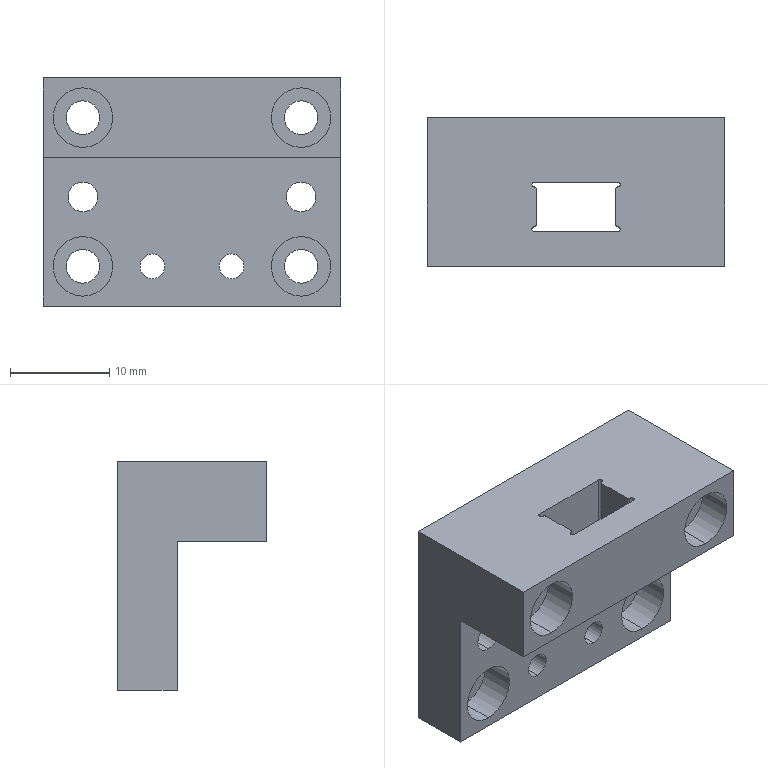Part | NX | features BREP 1 | 1 solid | 50 faces | box 30 x 15 x 23 mm | volume 5187 mm3 | cylinder 34 | plane 16 | commonest cylinder face diameters 3.4 x8 6 x8 0.5 x6 0.4 x4 2.5 x4 3 x4
STEP:
#1=CARTESIAN_POINT('',(4.45,-3.75,3.5));
#2=VERTEX_POINT('',#1);
#3=CARTESIAN_POINT('',(4.2,-3.5,3.5));
#4=VERTEX_POINT('',#3);
#5=CARTESIAN_POINT('',(4.2,-3.75,3.5));
#6=DIRECTION('',(0.,0.,1.));
#7=DIRECTION('',(1.,0.,0.));
#8=AXIS2_PLACEMENT_3D('',#5,#6,#7);
#9=CIRCLE('',#8,0.25);
#10=EDGE_CURVE('',#2,#4,#9,.T.);
#11=ORIENTED_EDGE('',*,*,#10,.F.);
#12=CARTESIAN_POINT('',(4.45,-3.75,11.5));
#13=VERTEX_POINT('',#12);
#14=CARTESIAN_POINT('',(4.45,-3.75,-11.5));
#15=DIRECTION('',(0.,0.,1.));
#16=VECTOR('',#15,1000.);
#17=LINE('',#14,#16);
#18=EDGE_CURVE('',#2,#13,#17,.T.);
#19=ORIENTED_EDGE('',*,*,#18,.T.);
#20=CARTESIAN_POINT('',(4.2,-3.5,11.5));
#21=VERTEX_POINT('',#20);
#22=CARTESIAN_POINT('',(4.2,-3.75,11.5));
#23=DIRECTION('',(0.,0.,1.));
#24=DIRECTION('',(1.,0.,0.));
#25=AXIS2_PLACEMENT_3D('',#22,#23,#24);
#26=CIRCLE('',#25,0.25);
#27=EDGE_CURVE('',#13,#21,#26,.T.);
#28=ORIENTED_EDGE('',*,*,#27,.T.);
#29=CARTESIAN_POINT('',(4.2,-3.5,-11.5));
#30=DIRECTION('',(0.,0.,1.));
#31=VECTOR('',#30,1000.);
#32=LINE('',#29,#31);
#33=EDGE_CURVE('',#4,#21,#32,.T.);
#34=ORIENTED_EDGE('',*,*,#33,.F.);
#35=EDGE_LOOP('',(#11,#19,#28,#34));
#36=FACE_BOUND('',#35,.T.);
#37=CARTESIAN_POINT('',(4.2,-3.75,-11.5));
#38=DIRECTION('',(0.,0.,1.));
#39=DIRECTION('',(-1.,0.,0.));
#40=AXIS2_PLACEMENT_3D('',#37,#38,#39);
#41=CYLINDRICAL_SURFACE('',#40,0.25);
#42=ADVANCED_FACE('',(#36),#41,.F.);
#43=CARTESIAN_POINT('',(4.45,0.75,3.5));
#44=VERTEX_POINT('',#43);
#45=CARTESIAN_POINT('',(4.2,1.,3.5));
#46=VERTEX_POINT('',#45);
#47=CARTESIAN_POINT('',(4.2,0.75,3.5));
#48=DIRECTION('',(0.,0.,1.));
#49=DIRECTION('',(1.,0.,0.));
#50=AXIS2_PLACEMENT_3D('',#47,#48,#49);
#51=CIRCLE('',#50,0.25);
#52=EDGE_CURVE('',#44,#46,#51,.T.);
#53=ORIENTED_EDGE('',*,*,#52,.F.);
#54=CARTESIAN_POINT('',(4.45,0.75,11.5));
#55=VERTEX_POINT('',#54);
#56=CARTESIAN_POINT('',(4.45,0.75,-11.5));
#57=DIRECTION('',(0.,0.,1.));
#58=VECTOR('',#57,1000.);
#59=LINE('',#56,#58);
#60=EDGE_CURVE('',#44,#55,#59,.T.);
#61=ORIENTED_EDGE('',*,*,#60,.T.);
#62=CARTESIAN_POINT('',(4.2,1.,11.5));
#63=VERTEX_POINT('',#62);
#64=CARTESIAN_POINT('',(4.2,0.75,11.5));
#65=DIRECTION('',(0.,0.,1.));
#66=DIRECTION('',(1.,0.,0.));
#67=AXIS2_PLACEMENT_3D('',#64,#65,#66);
#68=CIRCLE('',#67,0.25);
#69=EDGE_CURVE('',#55,#63,#68,.T.);
#70=ORIENTED_EDGE('',*,*,#69,.T.);
#71=CARTESIAN_POINT('',(4.2,1.,-11.5));
#72=DIRECTION('',(0.,0.,1.));
#73=VECTOR('',#72,1000.);
#74=LINE('',#71,#73);
#75=EDGE_CURVE('',#46,#63,#74,.T.);
#76=ORIENTED_EDGE('',*,*,#75,.F.);
#77=EDGE_LOOP('',(#53,#61,#70,#76));
#78=FACE_BOUND('',#77,.T.);
#79=CARTESIAN_POINT('',(4.2,0.75,-11.5));
#80=DIRECTION('',(0.,0.,1.));
#81=DIRECTION('',(-1.,0.,0.));
#82=AXIS2_PLACEMENT_3D('',#79,#80,#81);
#83=CYLINDRICAL_SURFACE('',#82,0.25);
#84=ADVANCED_FACE('',(#78),#83,.F.);
#85=CARTESIAN_POINT('',(4.,7.5,-6.25));
#86=VERTEX_POINT('',#85);
#87=CARTESIAN_POINT('',(4.,7.5,-8.75));
#88=VERTEX_POINT('',#87);
#89=CARTESIAN_POINT('',(4.,7.5,-7.5));
#90=DIRECTION('',(0.,-1.,0.));
#91=DIRECTION('',(0.,0.,-1.));
#92=AXIS2_PLACEMENT_3D('',#89,#90,#91);
#93=CIRCLE('',#92,1.25);
#94=EDGE_CURVE('',#86,#88,#93,.T.);
#95=ORIENTED_EDGE('',*,*,#94,.F.);
#96=CARTESIAN_POINT('',(4.,1.5,-6.25));
#97=VERTEX_POINT('',#96);
#98=CARTESIAN_POINT('',(4.,1.5,-6.25));
#99=DIRECTION('',(0.,-1.,0.));
#100=VECTOR('',#99,1000.);
#101=LINE('',#98,#100);
#102=EDGE_CURVE('',#97,#86,#101,.F.);
#103=ORIENTED_EDGE('',*,*,#102,.F.);
#104=CARTESIAN_POINT('',(4.,1.5,-8.75));
#105=VERTEX_POINT('',#104);
#106=CARTESIAN_POINT('',(4.,1.5,-7.5));
#107=DIRECTION('',(0.,-1.,0.));
#108=DIRECTION('',(0.,0.,-1.));
#109=AXIS2_PLACEMENT_3D('',#106,#107,#108);
#110=CIRCLE('',#109,1.25);
#111=EDGE_CURVE('',#97,#105,#110,.T.);
#112=ORIENTED_EDGE('',*,*,#111,.T.);
#113=CARTESIAN_POINT('',(4.,1.5,-8.75));
#114=DIRECTION('',(0.,-1.,0.));
#115=VECTOR('',#114,1000.);
#116=LINE('',#113,#115);
#117=EDGE_CURVE('',#105,#88,#116,.F.);
#118=ORIENTED_EDGE('',*,*,#117,.T.);
#119=EDGE_LOOP('',(#95,#103,#112,#118));
#120=FACE_BOUND('',#119,.T.);
#121=CARTESIAN_POINT('',(4.,1.5,-7.5));
#122=DIRECTION('',(0.,-1.,0.));
#123=DIRECTION('',(0.,0.,1.));
#124=AXIS2_PLACEMENT_3D('',#121,#122,#123);
#125=CYLINDRICAL_SURFACE('',#124,1.25);
#126=ADVANCED_FACE('',(#120),#125,.F.);
#127=CARTESIAN_POINT('',(-4.,7.5,-6.25));
#128=VERTEX_POINT('',#127);
#129=CARTESIAN_POINT('',(-4.,7.5,-8.75));
#130=VERTEX_POINT('',#129);
#131=CARTESIAN_POINT('',(-4.,7.5,-7.5));
#132=DIRECTION('',(0.,-1.,0.));
#133=DIRECTION('',(0.,0.,-1.));
#134=AXIS2_PLACEMENT_3D('',#131,#132,#133);
#135=CIRCLE('',#134,1.25);
#136=EDGE_CURVE('',#128,#130,#135,.T.);
#137=ORIENTED_EDGE('',*,*,#136,.F.);
#138=CARTESIAN_POINT('',(-4.,1.5,-6.25));
#139=VERTEX_POINT('',#138);
#140=CARTESIAN_POINT('',(-4.,1.5,-6.25));
#141=DIRECTION('',(0.,-1.,0.));
#142=VECTOR('',#141,1000.);
#143=LINE('',#140,#142);
#144=EDGE_CURVE('',#139,#128,#143,.F.);
#145=ORIENTED_EDGE('',*,*,#144,.F.);
#146=CARTESIAN_POINT('',(-4.,1.5,-8.75));
#147=VERTEX_POINT('',#146);
#148=CARTESIAN_POINT('',(-4.,1.5,-7.5));
#149=DIRECTION('',(0.,-1.,0.));
#150=DIRECTION('',(0.,0.,-1.));
#151=AXIS2_PLACEMENT_3D('',#148,#149,#150);
#152=CIRCLE('',#151,1.25);
#153=EDGE_CURVE('',#139,#147,#152,.T.);
#154=ORIENTED_EDGE('',*,*,#153,.T.);
#155=CARTESIAN_POINT('',(-4.,1.5,-8.75));
#156=DIRECTION('',(0.,-1.,0.));
#157=VECTOR('',#156,1000.);
#158=LINE('',#155,#157);
#159=EDGE_CURVE('',#147,#130,#158,.F.);
#160=ORIENTED_EDGE('',*,*,#159,.T.);
#161=EDGE_LOOP('',(#137,#145,#154,#160));
#162=FACE_BOUND('',#161,.T.);
#163=CARTESIAN_POINT('',(-4.,1.5,-7.5));
#164=DIRECTION('',(0.,-1.,0.));
#165=DIRECTION('',(0.,0.,1.));
#166=AXIS2_PLACEMENT_3D('',#163,#164,#165);
#167=CYLINDRICAL_SURFACE('',#166,1.25);
#168=ADVANCED_FACE('',(#162),#167,.F.);
#169=CARTESIAN_POINT('',(-11.,4.9,-4.5));
#170=VERTEX_POINT('',#169);
#171=CARTESIAN_POINT('',(-11.,4.9,-10.5));
#172=VERTEX_POINT('',#171);
#173=CARTESIAN_POINT('',(-11.,4.9,-7.5));
#174=DIRECTION('',(0.,-1.,0.));
#175=DIRECTION('',(0.,0.,-1.));
#176=AXIS2_PLACEMENT_3D('',#173,#174,#175);
#177=CIRCLE('',#176,3.);
#178=EDGE_CURVE('',#170,#172,#177,.T.);
#179=ORIENTED_EDGE('',*,*,#178,.F.);
#180=CARTESIAN_POINT('',(-11.,1.5,-4.5));
#181=VERTEX_POINT('',#180);
#182=CARTESIAN_POINT('',(-11.,1.5,-4.5));
#183=DIRECTION('',(0.,-1.,0.));
#184=VECTOR('',#183,1000.);
#185=LINE('',#182,#184);
#186=EDGE_CURVE('',#181,#170,#185,.F.);
#187=ORIENTED_EDGE('',*,*,#186,.F.);
#188=CARTESIAN_POINT('',(-11.,1.5,-10.5));
#189=VERTEX_POINT('',#188);
#190=CARTESIAN_POINT('',(-11.,1.5,-7.5));
#191=DIRECTION('',(0.,-1.,0.));
#192=DIRECTION('',(0.,0.,-1.));
#193=AXIS2_PLACEMENT_3D('',#190,#191,#192);
#194=CIRCLE('',#193,3.);
#195=EDGE_CURVE('',#181,#189,#194,.T.);
#196=ORIENTED_EDGE('',*,*,#195,.T.);
#197=CARTESIAN_POINT('',(-11.,1.5,-10.5));
#198=DIRECTION('',(0.,-1.,0.));
#199=VECTOR('',#198,1000.);
#200=LINE('',#197,#199);
#201=EDGE_CURVE('',#189,#172,#200,.F.);
#202=ORIENTED_EDGE('',*,*,#201,.T.);
#203=EDGE_LOOP('',(#179,#187,#196,#202));
#204=FACE_BOUND('',#203,.T.);
#205=CARTESIAN_POINT('',(-11.,1.5,-7.5));
#206=DIRECTION('',(0.,-1.,0.));
#207=DIRECTION('',(0.,0.,1.));
#208=AXIS2_PLACEMENT_3D('',#205,#206,#207);
#209=CYLINDRICAL_SURFACE('',#208,3.);
#210=ADVANCED_FACE('',(#204),#209,.F.);
#211=CARTESIAN_POINT('',(-11.,7.5,-5.8));
#212=VERTEX_POINT('',#211);
#213=CARTESIAN_POINT('',(-11.,7.5,-9.2));
#214=VERTEX_POINT('',#213);
#215=CARTESIAN_POINT('',(-11.,7.5,-7.5));
#216=DIRECTION('',(0.,-1.,0.));
#217=DIRECTION('',(0.,0.,-1.));
#218=AXIS2_PLACEMENT_3D('',#215,#216,#217);
#219=CIRCLE('',#218,1.7);
#220=EDGE_CURVE('',#212,#214,#219,.T.);
#221=ORIENTED_EDGE('',*,*,#220,.F.);
#222=CARTESIAN_POINT('',(-11.,4.9,-5.8));
#223=VERTEX_POINT('',#222);
#224=CARTESIAN_POINT('',(-11.,1.5,-5.8));
#225=DIRECTION('',(0.,-1.,0.));
#226=VECTOR('',#225,1000.);
#227=LINE('',#224,#226);
#228=EDGE_CURVE('',#223,#212,#227,.F.);
#229=ORIENTED_EDGE('',*,*,#228,.F.);
#230=CARTESIAN_POINT('',(-11.,4.9,-9.2));
#231=VERTEX_POINT('',#230);
#232=CARTESIAN_POINT('',(-11.,4.9,-7.5));
#233=DIRECTION('',(0.,-1.,0.));
#234=DIRECTION('',(0.,0.,-1.));
#235=AXIS2_PLACEMENT_3D('',#232,#233,#234);
#236=CIRCLE('',#235,1.7);
#237=EDGE_CURVE('',#223,#231,#236,.T.);
#238=ORIENTED_EDGE('',*,*,#237,.T.);
#239=CARTESIAN_POINT('',(-11.,1.5,-9.2));
#240=DIRECTION('',(0.,-1.,0.));
#241=VECTOR('',#240,1000.);
#242=LINE('',#239,#241);
#243=EDGE_CURVE('',#231,#214,#242,.F.);
#244=ORIENTED_EDGE('',*,*,#243,.T.);
#245=EDGE_LOOP('',(#221,#229,#238,#244));
#246=FACE_BOUND('',#245,.T.);
#247=CARTESIAN_POINT('',(-11.,1.5,-7.5));
#248=DIRECTION('',(0.,-1.,0.));
#249=DIRECTION('',(0.,0.,1.));
#250=AXIS2_PLACEMENT_3D('',#247,#248,#249);
#251=CYLINDRICAL_SURFACE('',#250,1.7);
#252=ADVANCED_FACE('',(#246),#251,.F.);
#253=CARTESIAN_POINT('',(11.,4.9,-4.5));
#254=VERTEX_POINT('',#253);
#255=CARTESIAN_POINT('',(11.,4.9,-10.5));
#256=VERTEX_POINT('',#255);
#257=CARTESIAN_POINT('',(11.,4.9,-7.5));
#258=DIRECTION('',(0.,-1.,0.));
#259=DIRECTION('',(0.,0.,-1.));
#260=AXIS2_PLACEMENT_3D('',#257,#258,#259);
#261=CIRCLE('',#260,3.);
#262=EDGE_CURVE('',#254,#256,#261,.T.);
#263=ORIENTED_EDGE('',*,*,#262,.F.);
#264=CARTESIAN_POINT('',(11.,1.5,-4.5));
#265=VERTEX_POINT('',#264);
#266=CARTESIAN_POINT('',(11.,1.5,-4.5));
#267=DIRECTION('',(0.,-1.,0.));
#268=VECTOR('',#267,1000.);
#269=LINE('',#266,#268);
#270=EDGE_CURVE('',#265,#254,#269,.F.);
#271=ORIENTED_EDGE('',*,*,#270,.F.);
#272=CARTESIAN_POINT('',(11.,1.5,-10.5));
#273=VERTEX_POINT('',#272);
#274=CARTESIAN_POINT('',(11.,1.5,-7.5));
#275=DIRECTION('',(0.,-1.,0.));
#276=DIRECTION('',(0.,0.,-1.));
#277=AXIS2_PLACEMENT_3D('',#274,#275,#276);
#278=CIRCLE('',#277,3.);
#279=EDGE_CURVE('',#265,#273,#278,.T.);
#280=ORIENTED_EDGE('',*,*,#279,.T.);
#281=CARTESIAN_POINT('',(11.,1.5,-10.5));
#282=DIRECTION('',(0.,-1.,0.));
#283=VECTOR('',#282,1000.);
#284=LINE('',#281,#283);
#285=EDGE_CURVE('',#273,#256,#284,.F.);
#286=ORIENTED_EDGE('',*,*,#285,.T.);
#287=EDGE_LOOP('',(#263,#271,#280,#286));
#288=FACE_BOUND('',#287,.T.);
#289=CARTESIAN_POINT('',(11.,1.5,-7.5));
#290=DIRECTION('',(0.,-1.,0.));
#291=DIRECTION('',(0.,0.,1.));
#292=AXIS2_PLACEMENT_3D('',#289,#290,#291);
#293=CYLINDRICAL_SURFACE('',#292,3.);
#294=ADVANCED_FACE('',(#288),#293,.F.);
#295=CARTESIAN_POINT('',(11.,7.5,-5.8));
#296=VERTEX_POINT('',#295);
#297=CARTESIAN_POINT('',(11.,7.5,-9.2));
#298=VERTEX_POINT('',#297);
#299=CARTESIAN_POINT('',(11.,7.5,-7.5));
#300=DIRECTION('',(0.,-1.,0.));
#301=DIRECTION('',(0.,0.,-1.));
#302=AXIS2_PLACEMENT_3D('',#299,#300,#301);
#303=CIRCLE('',#302,1.7);
#304=EDGE_CURVE('',#296,#298,#303,.T.);
#305=ORIENTED_EDGE('',*,*,#304,.F.);
#306=CARTESIAN_POINT('',(11.,4.9,-5.8));
#307=VERTEX_POINT('',#306);
#308=CARTESIAN_POINT('',(11.,1.5,-5.8));
#309=DIRECTION('',(0.,-1.,0.));
#310=VECTOR('',#309,1000.);
#311=LINE('',#308,#310);
#312=EDGE_CURVE('',#307,#296,#311,.F.);
#313=ORIENTED_EDGE('',*,*,#312,.F.);
#314=CARTESIAN_POINT('',(11.,4.9,-9.2));
#315=VERTEX_POINT('',#314);
#316=CARTESIAN_POINT('',(11.,4.9,-7.5));
#317=DIRECTION('',(0.,-1.,0.));
#318=DIRECTION('',(0.,0.,-1.));
#319=AXIS2_PLACEMENT_3D('',#316,#317,#318);
#320=CIRCLE('',#319,1.7);
#321=EDGE_CURVE('',#307,#315,#320,.T.);
#322=ORIENTED_EDGE('',*,*,#321,.T.);
#323=CARTESIAN_POINT('',(11.,1.5,-9.2));
#324=DIRECTION('',(0.,-1.,0.));
#325=VECTOR('',#324,1000.);
#326=LINE('',#323,#325);
#327=EDGE_CURVE('',#315,#298,#326,.F.);
#328=ORIENTED_EDGE('',*,*,#327,.T.);
#329=EDGE_LOOP('',(#305,#313,#322,#328));
#330=FACE_BOUND('',#329,.T.);
#331=CARTESIAN_POINT('',(11.,1.5,-7.5));
#332=DIRECTION('',(0.,-1.,0.));
#333=DIRECTION('',(0.,0.,1.));
#334=AXIS2_PLACEMENT_3D('',#331,#332,#333);
#335=CYLINDRICAL_SURFACE('',#334,1.7);
#336=ADVANCED_FACE('',(#330),#335,.F.);
#337=CARTESIAN_POINT('',(-11.,7.5,1.));
#338=VERTEX_POINT('',#337);
#339=CARTESIAN_POINT('',(-11.,7.5,-2.));
#340=VERTEX_POINT('',#339);
#341=CARTESIAN_POINT('',(-11.,7.5,-0.5));
#342=DIRECTION('',(0.,-1.,0.));
#343=DIRECTION('',(0.,0.,-1.));
#344=AXIS2_PLACEMENT_3D('',#341,#342,#343);
#345=CIRCLE('',#344,1.5);
#346=EDGE_CURVE('',#338,#340,#345,.T.);
#347=ORIENTED_EDGE('',*,*,#346,.F.);
#348=CARTESIAN_POINT('',(-11.,1.5,1.));
#349=VERTEX_POINT('',#348);
#350=CARTESIAN_POINT('',(-11.,-7.5,1.));
#351=DIRECTION('',(0.,-1.,0.));
#352=VECTOR('',#351,1000.);
#353=LINE('',#350,#352);
#354=EDGE_CURVE('',#349,#338,#353,.F.);
#355=ORIENTED_EDGE('',*,*,#354,.F.);
#356=CARTESIAN_POINT('',(-11.,1.5,-2.));
#357=VERTEX_POINT('',#356);
#358=CARTESIAN_POINT('',(-11.,1.5,-0.5));
#359=DIRECTION('',(0.,1.,0.));
#360=DIRECTION('',(-1.,0.,0.));
#361=AXIS2_PLACEMENT_3D('',#358,#359,#360);
#362=CIRCLE('',#361,1.5);
#363=EDGE_CURVE('',#357,#349,#362,.T.);
#364=ORIENTED_EDGE('',*,*,#363,.F.);
#365=CARTESIAN_POINT('',(-11.,-7.5,-2.));
#366=DIRECTION('',(0.,-1.,0.));
#367=VECTOR('',#366,1000.);
#368=LINE('',#365,#367);
#369=EDGE_CURVE('',#357,#340,#368,.F.);
#370=ORIENTED_EDGE('',*,*,#369,.T.);
#371=EDGE_LOOP('',(#347,#355,#364,#370));
#372=FACE_BOUND('',#371,.T.);
#373=CARTESIAN_POINT('',(-11.,-7.5,-0.5));
#374=DIRECTION('',(0.,-1.,0.));
#375=DIRECTION('',(0.,0.,1.));
#376=AXIS2_PLACEMENT_3D('',#373,#374,#375);
#377=CYLINDRICAL_SURFACE('',#376,1.5);
#378=ADVANCED_FACE('',(#372),#377,.F.);
#379=CARTESIAN_POINT('',(11.,7.5,1.));
#380=VERTEX_POINT('',#379);
#381=CARTESIAN_POINT('',(11.,7.5,-2.));
#382=VERTEX_POINT('',#381);
#383=CARTESIAN_POINT('',(11.,7.5,-0.5));
#384=DIRECTION('',(0.,-1.,0.));
#385=DIRECTION('',(0.,0.,-1.));
#386=AXIS2_PLACEMENT_3D('',#383,#384,#385);
#387=CIRCLE('',#386,1.5);
#388=EDGE_CURVE('',#380,#382,#387,.T.);
#389=ORIENTED_EDGE('',*,*,#388,.F.);
#390=CARTESIAN_POINT('',(11.,1.5,1.));
#391=VERTEX_POINT('',#390);
#392=CARTESIAN_POINT('',(11.,-7.5,1.));
#393=DIRECTION('',(0.,-1.,0.));
#394=VECTOR('',#393,1000.);
#395=LINE('',#392,#394);
#396=EDGE_CURVE('',#391,#380,#395,.F.);
#397=ORIENTED_EDGE('',*,*,#396,.F.);
#398=CARTESIAN_POINT('',(11.,1.5,-2.));
#399=VERTEX_POINT('',#398);
#400=CARTESIAN_POINT('',(11.,1.5,-0.5));
#401=DIRECTION('',(0.,1.,0.));
#402=DIRECTION('',(-1.,0.,0.));
#403=AXIS2_PLACEMENT_3D('',#400,#401,#402);
#404=CIRCLE('',#403,1.5);
#405=EDGE_CURVE('',#399,#391,#404,.T.);
#406=ORIENTED_EDGE('',*,*,#405,.F.);
#407=CARTESIAN_POINT('',(11.,-7.5,-2.));
#408=DIRECTION('',(0.,-1.,0.));
#409=VECTOR('',#408,1000.);
#410=LINE('',#407,#409);
#411=EDGE_CURVE('',#399,#382,#410,.F.);
#412=ORIENTED_EDGE('',*,*,#411,.T.);
#413=EDGE_LOOP('',(#389,#397,#406,#412));
#414=FACE_BOUND('',#413,.T.);
#415=CARTESIAN_POINT('',(11.,-7.5,-0.5));
#416=DIRECTION('',(0.,-1.,0.));
#417=DIRECTION('',(0.,0.,1.));
#418=AXIS2_PLACEMENT_3D('',#415,#416,#417);
#419=CYLINDRICAL_SURFACE('',#418,1.5);
#420=ADVANCED_FACE('',(#414),#419,.F.);
#421=CARTESIAN_POINT('',(-11.,-4.1,10.5));
#422=VERTEX_POINT('',#421);
#423=CARTESIAN_POINT('',(-11.,-4.1,4.5));
#424=VERTEX_POINT('',#423);
#425=CARTESIAN_POINT('',(-11.,-4.1,7.5));
#426=DIRECTION('',(0.,-1.,0.));
#427=DIRECTION('',(0.,0.,-1.));
#428=AXIS2_PLACEMENT_3D('',#425,#426,#427);
#429=CIRCLE('',#428,3.);
#430=EDGE_CURVE('',#422,#424,#429,.T.);
#431=ORIENTED_EDGE('',*,*,#430,.F.);
#432=CARTESIAN_POINT('',(-11.,-7.5,10.5));
#433=VERTEX_POINT('',#432);
#434=CARTESIAN_POINT('',(-11.,-7.5,10.5));
#435=DIRECTION('',(0.,-1.,0.));
#436=VECTOR('',#435,1000.);
#437=LINE('',#434,#436);
#438=EDGE_CURVE('',#433,#422,#437,.F.);
#439=ORIENTED_EDGE('',*,*,#438,.F.);
#440=CARTESIAN_POINT('',(-11.,-7.5,4.5));
#441=VERTEX_POINT('',#440);
#442=CARTESIAN_POINT('',(-11.,-7.5,7.5));
#443=DIRECTION('',(0.,-1.,0.));
#444=DIRECTION('',(0.,0.,-1.));
#445=AXIS2_PLACEMENT_3D('',#442,#443,#444);
#446=CIRCLE('',#445,3.);
#447=EDGE_CURVE('',#433,#441,#446,.T.);
#448=ORIENTED_EDGE('',*,*,#447,.T.);
#449=CARTESIAN_POINT('',(-11.,-7.5,4.5));
#450=DIRECTION('',(0.,-1.,0.));
#451=VECTOR('',#450,1000.);
#452=LINE('',#449,#451);
#453=EDGE_CURVE('',#441,#424,#452,.F.);
#454=ORIENTED_EDGE('',*,*,#453,.T.);
#455=EDGE_LOOP('',(#431,#439,#448,#454));
#456=FACE_BOUND('',#455,.T.);
#457=CARTESIAN_POINT('',(-11.,-7.5,7.5));
#458=DIRECTION('',(0.,-1.,0.));
#459=DIRECTION('',(0.,0.,1.));
#460=AXIS2_PLACEMENT_3D('',#457,#458,#459);
#461=CYLINDRICAL_SURFACE('',#460,3.);
#462=ADVANCED_FACE('',(#456),#461,.F.);
#463=CARTESIAN_POINT('',(-11.,7.5,9.2));
#464=VERTEX_POINT('',#463);
#465=CARTESIAN_POINT('',(-11.,7.5,5.8));
#466=VERTEX_POINT('',#465);
#467=CARTESIAN_POINT('',(-11.,7.5,7.5));
#468=DIRECTION('',(0.,-1.,0.));
#469=DIRECTION('',(0.,0.,-1.));
#470=AXIS2_PLACEMENT_3D('',#467,#468,#469);
#471=CIRCLE('',#470,1.7);
#472=EDGE_CURVE('',#464,#466,#471,.T.);
#473=ORIENTED_EDGE('',*,*,#472,.F.);
#474=CARTESIAN_POINT('',(-11.,-4.1,9.2));
#475=VERTEX_POINT('',#474);
#476=CARTESIAN_POINT('',(-11.,-7.5,9.2));
#477=DIRECTION('',(0.,-1.,0.));
#478=VECTOR('',#477,1000.);
#479=LINE('',#476,#478);
#480=EDGE_CURVE('',#475,#464,#479,.F.);
#481=ORIENTED_EDGE('',*,*,#480,.F.);
#482=CARTESIAN_POINT('',(-11.,-4.1,5.8));
#483=VERTEX_POINT('',#482);
#484=CARTESIAN_POINT('',(-11.,-4.1,7.5));
#485=DIRECTION('',(0.,-1.,0.));
#486=DIRECTION('',(0.,0.,-1.));
#487=AXIS2_PLACEMENT_3D('',#484,#485,#486);
#488=CIRCLE('',#487,1.7);
#489=EDGE_CURVE('',#475,#483,#488,.T.);
#490=ORIENTED_EDGE('',*,*,#489,.T.);
#491=CARTESIAN_POINT('',(-11.,-7.5,5.8));
#492=DIRECTION('',(0.,-1.,0.));
#493=VECTOR('',#492,1000.);
#494=LINE('',#491,#493);
#495=EDGE_CURVE('',#483,#466,#494,.F.);
#496=ORIENTED_EDGE('',*,*,#495,.T.);
#497=EDGE_LOOP('',(#473,#481,#490,#496));
#498=FACE_BOUND('',#497,.T.);
#499=CARTESIAN_POINT('',(-11.,-7.5,7.5));
#500=DIRECTION('',(0.,-1.,0.));
#501=DIRECTION('',(0.,0.,1.));
#502=AXIS2_PLACEMENT_3D('',#499,#500,#501);
#503=CYLINDRICAL_SURFACE('',#502,1.7);
#504=ADVANCED_FACE('',(#498),#503,.F.);
#505=CARTESIAN_POINT('',(11.,-4.1,10.5));
#506=VERTEX_POINT('',#505);
#507=CARTESIAN_POINT('',(11.,-4.1,4.5));
#508=VERTEX_POINT('',#507);
#509=CARTESIAN_POINT('',(11.,-4.1,7.5));
#510=DIRECTION('',(0.,-1.,0.));
#511=DIRECTION('',(0.,0.,-1.));
#512=AXIS2_PLACEMENT_3D('',#509,#510,#511);
#513=CIRCLE('',#512,3.);
#514=EDGE_CURVE('',#506,#508,#513,.T.);
#515=ORIENTED_EDGE('',*,*,#514,.F.);
#516=CARTESIAN_POINT('',(11.,-7.5,10.5));
#517=VERTEX_POINT('',#516);
#518=CARTESIAN_POINT('',(11.,-7.5,10.5));
#519=DIRECTION('',(0.,-1.,0.));
#520=VECTOR('',#519,1000.);
#521=LINE('',#518,#520);
#522=EDGE_CURVE('',#517,#506,#521,.F.);
#523=ORIENTED_EDGE('',*,*,#522,.F.);
#524=CARTESIAN_POINT('',(11.,-7.5,4.5));
#525=VERTEX_POINT('',#524);
#526=CARTESIAN_POINT('',(11.,-7.5,7.5));
#527=DIRECTION('',(0.,-1.,0.));
#528=DIRECTION('',(0.,0.,-1.));
#529=AXIS2_PLACEMENT_3D('',#526,#527,#528);
#530=CIRCLE('',#529,3.);
#531=EDGE_CURVE('',#517,#525,#530,.T.);
#532=ORIENTED_EDGE('',*,*,#531,.T.);
#533=CARTESIAN_POINT('',(11.,-7.5,4.5));
#534=DIRECTION('',(0.,-1.,0.));
#535=VECTOR('',#534,1000.);
#536=LINE('',#533,#535);
#537=EDGE_CURVE('',#525,#508,#536,.F.);
#538=ORIENTED_EDGE('',*,*,#537,.T.);
#539=EDGE_LOOP('',(#515,#523,#532,#538));
#540=FACE_BOUND('',#539,.T.);
#541=CARTESIAN_POINT('',(11.,-7.5,7.5));
#542=DIRECTION('',(0.,-1.,0.));
#543=DIRECTION('',(0.,0.,1.));
#544=AXIS2_PLACEMENT_3D('',#541,#542,#543);
#545=CYLINDRICAL_SURFACE('',#544,3.);
#546=ADVANCED_FACE('',(#540),#545,.F.);
#547=CARTESIAN_POINT('',(11.,7.5,9.2));
#548=VERTEX_POINT('',#547);
#549=CARTESIAN_POINT('',(11.,7.5,5.8));
#550=VERTEX_POINT('',#549);
#551=CARTESIAN_POINT('',(11.,7.5,7.5));
#552=DIRECTION('',(0.,-1.,0.));
#553=DIRECTION('',(0.,0.,-1.));
#554=AXIS2_PLACEMENT_3D('',#551,#552,#553);
#555=CIRCLE('',#554,1.7);
#556=EDGE_CURVE('',#548,#550,#555,.T.);
#557=ORIENTED_EDGE('',*,*,#556,.F.);
#558=CARTESIAN_POINT('',(11.,-4.1,9.2));
#559=VERTEX_POINT('',#558);
#560=CARTESIAN_POINT('',(11.,-7.5,9.2));
#561=DIRECTION('',(0.,-1.,0.));
#562=VECTOR('',#561,1000.);
#563=LINE('',#560,#562);
#564=EDGE_CURVE('',#559,#548,#563,.F.);
#565=ORIENTED_EDGE('',*,*,#564,.F.);
#566=CARTESIAN_POINT('',(11.,-4.1,5.8));
#567=VERTEX_POINT('',#566);
#568=CARTESIAN_POINT('',(11.,-4.1,7.5));
#569=DIRECTION('',(0.,-1.,0.));
#570=DIRECTION('',(0.,0.,-1.));
#571=AXIS2_PLACEMENT_3D('',#568,#569,#570);
#572=CIRCLE('',#571,1.7);
#573=EDGE_CURVE('',#559,#567,#572,.T.);
#574=ORIENTED_EDGE('',*,*,#573,.T.);
#575=CARTESIAN_POINT('',(11.,-7.5,5.8));
#576=DIRECTION('',(0.,-1.,0.));
#577=VECTOR('',#576,1000.);
#578=LINE('',#575,#577);
#579=EDGE_CURVE('',#567,#550,#578,.F.);
#580=ORIENTED_EDGE('',*,*,#579,.T.);
#581=EDGE_LOOP('',(#557,#565,#574,#580));
#582=FACE_BOUND('',#581,.T.);
#583=CARTESIAN_POINT('',(11.,-7.5,7.5));
#584=DIRECTION('',(0.,-1.,0.));
#585=DIRECTION('',(0.,0.,1.));
#586=AXIS2_PLACEMENT_3D('',#583,#584,#585);
#587=CYLINDRICAL_SURFACE('',#586,1.7);
#588=ADVANCED_FACE('',(#582),#587,.F.);
#589=CARTESIAN_POINT('',(-15.,1.5,-11.5));
#590=VERTEX_POINT('',#589);
#591=CARTESIAN_POINT('',(-15.,1.5,3.5));
#592=VERTEX_POINT('',#591);
#593=CARTESIAN_POINT('',(-15.,1.5,-11.5));
#594=DIRECTION('',(0.,0.,1.));
#595=VECTOR('',#594,1000.);
#596=LINE('',#593,#595);
#597=EDGE_CURVE('',#590,#592,#596,.T.);
#598=ORIENTED_EDGE('',*,*,#597,.T.);
#599=CARTESIAN_POINT('',(-15.,-7.5,3.5));
#600=VERTEX_POINT('',#599);
#601=CARTESIAN_POINT('',(-15.,-7.5,3.5));
#602=DIRECTION('',(0.,-1.,0.));
#603=VECTOR('',#602,1000.);
#604=LINE('',#601,#603);
#605=EDGE_CURVE('',#592,#600,#604,.T.);
#606=ORIENTED_EDGE('',*,*,#605,.T.);
#607=CARTESIAN_POINT('',(-15.,-7.5,11.5));
#608=VERTEX_POINT('',#607);
#609=CARTESIAN_POINT('',(-15.,-7.5,11.5));
#610=DIRECTION('',(0.,0.,-1.));
#611=VECTOR('',#610,1000.);
#612=LINE('',#609,#611);
#613=EDGE_CURVE('',#608,#600,#612,.T.);
#614=ORIENTED_EDGE('',*,*,#613,.F.);
#615=CARTESIAN_POINT('',(-15.,7.5,11.5));
#616=VERTEX_POINT('',#615);
#617=CARTESIAN_POINT('',(-15.,7.5,11.5));
#618=DIRECTION('',(0.,-1.,0.));
#619=VECTOR('',#618,1000.);
#620=LINE('',#617,#619);
#621=EDGE_CURVE('',#616,#608,#620,.T.);
#622=ORIENTED_EDGE('',*,*,#621,.F.);
#623=CARTESIAN_POINT('',(-15.,7.5,-11.5));
#624=VERTEX_POINT('',#623);
#625=CARTESIAN_POINT('',(-15.,7.5,11.5));
#626=DIRECTION('',(0.,0.,-1.));
#627=VECTOR('',#626,1000.);
#628=LINE('',#625,#627);
#629=EDGE_CURVE('',#616,#624,#628,.T.);
#630=ORIENTED_EDGE('',*,*,#629,.T.);
#631=CARTESIAN_POINT('',(-15.,7.5,-11.5));
#632=DIRECTION('',(0.,-1.,0.));
#633=VECTOR('',#632,1000.);
#634=LINE('',#631,#633);
#635=EDGE_CURVE('',#624,#590,#634,.T.);
#636=ORIENTED_EDGE('',*,*,#635,.T.);
#637=EDGE_LOOP('',(#598,#606,#614,#622,#630,#636));
#638=FACE_BOUND('',#637,.T.);
#639=CARTESIAN_POINT('',(-15.,7.5,11.5));
#640=DIRECTION('',(1.,0.,0.));
#641=DIRECTION('',(0.,0.,1.));
#642=AXIS2_PLACEMENT_3D('',#639,#640,#641);
#643=PLANE('',#642);
#644=ADVANCED_FACE('',(#638),#643,.F.);
#645=CARTESIAN_POINT('',(-11.,-7.5,7.5));
#646=DIRECTION('',(0.,-1.,0.));
#647=DIRECTION('',(0.,0.,-1.));
#648=AXIS2_PLACEMENT_3D('',#645,#646,#647);
#649=CIRCLE('',#648,3.);
#650=EDGE_CURVE('',#441,#433,#649,.T.);
#651=ORIENTED_EDGE('',*,*,#650,.F.);
#652=ORIENTED_EDGE('',*,*,#447,.F.);
#653=EDGE_LOOP('',(#651,#652));
#654=FACE_BOUND('',#653,.T.);
#655=CARTESIAN_POINT('',(11.,-7.5,7.5));
#656=DIRECTION('',(0.,-1.,0.));
#657=DIRECTION('',(0.,0.,-1.));
#658=AXIS2_PLACEMENT_3D('',#655,#656,#657);
#659=CIRCLE('',#658,3.);
#660=EDGE_CURVE('',#525,#517,#659,.T.);
#661=ORIENTED_EDGE('',*,*,#660,.F.);
#662=ORIENTED_EDGE('',*,*,#531,.F.);
#663=EDGE_LOOP('',(#661,#662));
#664=FACE_BOUND('',#663,.T.);
#665=ORIENTED_EDGE('',*,*,#613,.T.);
#666=CARTESIAN_POINT('',(15.,-7.5,3.5));
#667=VERTEX_POINT('',#666);
#668=CARTESIAN_POINT('',(-15.,-7.5,3.5));
#669=DIRECTION('',(1.,0.,0.));
#670=VECTOR('',#669,1000.);
#671=LINE('',#668,#670);
#672=EDGE_CURVE('',#600,#667,#671,.T.);
#673=ORIENTED_EDGE('',*,*,#672,.T.);
#674=CARTESIAN_POINT('',(15.,-7.5,11.5));
#675=VERTEX_POINT('',#674);
#676=CARTESIAN_POINT('',(15.,-7.5,11.5));
#677=DIRECTION('',(0.,0.,-1.));
#678=VECTOR('',#677,1000.);
#679=LINE('',#676,#678);
#680=EDGE_CURVE('',#675,#667,#679,.T.);
#681=ORIENTED_EDGE('',*,*,#680,.F.);
#682=CARTESIAN_POINT('',(-15.,-7.5,11.5));
#683=DIRECTION('',(1.,0.,0.));
#684=VECTOR('',#683,1000.);
#685=LINE('',#682,#684);
#686=EDGE_CURVE('',#608,#675,#685,.T.);
#687=ORIENTED_EDGE('',*,*,#686,.F.);
#688=EDGE_LOOP('',(#665,#673,#681,#687));
#689=FACE_BOUND('',#688,.T.);
#690=CARTESIAN_POINT('',(-15.,-7.5,11.5));
#691=DIRECTION('',(0.,1.,0.));
#692=DIRECTION('',(0.,0.,-1.));
#693=AXIS2_PLACEMENT_3D('',#690,#691,#692);
#694=PLANE('',#693);
#695=ADVANCED_FACE('',(#654,#664,#689),#694,.F.);
#696=CARTESIAN_POINT('',(15.,1.5,3.5));
#697=VERTEX_POINT('',#696);
#698=CARTESIAN_POINT('',(15.,-7.5,3.5));
#699=DIRECTION('',(0.,-1.,0.));
#700=VECTOR('',#699,1000.);
#701=LINE('',#698,#700);
#702=EDGE_CURVE('',#697,#667,#701,.T.);
#703=ORIENTED_EDGE('',*,*,#702,.F.);
#704=CARTESIAN_POINT('',(15.,1.5,-11.5));
#705=VERTEX_POINT('',#704);
#706=CARTESIAN_POINT('',(15.,1.5,-11.5));
#707=DIRECTION('',(0.,0.,1.));
#708=VECTOR('',#707,1000.);
#709=LINE('',#706,#708);
#710=EDGE_CURVE('',#705,#697,#709,.T.);
#711=ORIENTED_EDGE('',*,*,#710,.F.);
#712=CARTESIAN_POINT('',(15.,7.5,-11.5));
#713=VERTEX_POINT('',#712);
#714=CARTESIAN_POINT('',(15.,7.5,-11.5));
#715=DIRECTION('',(0.,-1.,0.));
#716=VECTOR('',#715,1000.);
#717=LINE('',#714,#716);
#718=EDGE_CURVE('',#713,#705,#717,.T.);
#719=ORIENTED_EDGE('',*,*,#718,.F.);
#720=CARTESIAN_POINT('',(15.,7.5,11.5));
#721=VERTEX_POINT('',#720);
#722=CARTESIAN_POINT('',(15.,7.5,11.5));
#723=DIRECTION('',(0.,0.,-1.));
#724=VECTOR('',#723,1000.);
#725=LINE('',#722,#724);
#726=EDGE_CURVE('',#721,#713,#725,.T.);
#727=ORIENTED_EDGE('',*,*,#726,.F.);
#728=CARTESIAN_POINT('',(15.,7.5,11.5));
#729=DIRECTION('',(0.,-1.,0.));
#730=VECTOR('',#729,1000.);
#731=LINE('',#728,#730);
#732=EDGE_CURVE('',#721,#675,#731,.T.);
#733=ORIENTED_EDGE('',*,*,#732,.T.);
#734=ORIENTED_EDGE('',*,*,#680,.T.);
#735=EDGE_LOOP('',(#703,#711,#719,#727,#733,#734));
#736=FACE_BOUND('',#735,.T.);
#737=CARTESIAN_POINT('',(15.,7.5,11.5));
#738=DIRECTION('',(1.,0.,0.));
#739=DIRECTION('',(0.,-1.,0.));
#740=AXIS2_PLACEMENT_3D('',#737,#738,#739);
#741=PLANE('',#740);
#742=ADVANCED_FACE('',(#736),#741,.T.);
#743=CARTESIAN_POINT('',(4.,7.5,-7.5));
#744=DIRECTION('',(0.,-1.,0.));
#745=DIRECTION('',(0.,0.,-1.));
#746=AXIS2_PLACEMENT_3D('',#743,#744,#745);
#747=CIRCLE('',#746,1.25);
#748=EDGE_CURVE('',#88,#86,#747,.T.);
#749=ORIENTED_EDGE('',*,*,#748,.T.);
#750=ORIENTED_EDGE('',*,*,#94,.T.);
#751=EDGE_LOOP('',(#749,#750));
#752=FACE_BOUND('',#751,.T.);
#753=CARTESIAN_POINT('',(-4.,7.5,-7.5));
#754=DIRECTION('',(0.,-1.,0.));
#755=DIRECTION('',(0.,0.,-1.));
#756=AXIS2_PLACEMENT_3D('',#753,#754,#755);
#757=CIRCLE('',#756,1.25);
#758=EDGE_CURVE('',#130,#128,#757,.T.);
#759=ORIENTED_EDGE('',*,*,#758,.T.);
#760=ORIENTED_EDGE('',*,*,#136,.T.);
#761=EDGE_LOOP('',(#759,#760));
#762=FACE_BOUND('',#761,.T.);
#763=CARTESIAN_POINT('',(-11.,7.5,-7.5));
#764=DIRECTION('',(0.,-1.,0.));
#765=DIRECTION('',(0.,0.,-1.));
#766=AXIS2_PLACEMENT_3D('',#763,#764,#765);
#767=CIRCLE('',#766,1.7);
#768=EDGE_CURVE('',#214,#212,#767,.T.);
#769=ORIENTED_EDGE('',*,*,#768,.T.);
#770=ORIENTED_EDGE('',*,*,#220,.T.);
#771=EDGE_LOOP('',(#769,#770));
#772=FACE_BOUND('',#771,.T.);
#773=CARTESIAN_POINT('',(11.,7.5,-7.5));
#774=DIRECTION('',(0.,-1.,0.));
#775=DIRECTION('',(0.,0.,-1.));
#776=AXIS2_PLACEMENT_3D('',#773,#774,#775);
#777=CIRCLE('',#776,1.7);
#778=EDGE_CURVE('',#298,#296,#777,.T.);
#779=ORIENTED_EDGE('',*,*,#778,.T.);
#780=ORIENTED_EDGE('',*,*,#304,.T.);
#781=EDGE_LOOP('',(#779,#780));
#782=FACE_BOUND('',#781,.T.);
#783=CARTESIAN_POINT('',(-11.,7.5,-0.5));
#784=DIRECTION('',(0.,-1.,0.));
#785=DIRECTION('',(0.,0.,-1.));
#786=AXIS2_PLACEMENT_3D('',#783,#784,#785);
#787=CIRCLE('',#786,1.5);
#788=EDGE_CURVE('',#340,#338,#787,.T.);
#789=ORIENTED_EDGE('',*,*,#788,.T.);
#790=ORIENTED_EDGE('',*,*,#346,.T.);
#791=EDGE_LOOP('',(#789,#790));
#792=FACE_BOUND('',#791,.T.);
#793=CARTESIAN_POINT('',(11.,7.5,-0.5));
#794=DIRECTION('',(0.,-1.,0.));
#795=DIRECTION('',(0.,0.,-1.));
#796=AXIS2_PLACEMENT_3D('',#793,#794,#795);
#797=CIRCLE('',#796,1.5);
#798=EDGE_CURVE('',#382,#380,#797,.T.);
#799=ORIENTED_EDGE('',*,*,#798,.T.);
#800=ORIENTED_EDGE('',*,*,#388,.T.);
#801=EDGE_LOOP('',(#799,#800));
#802=FACE_BOUND('',#801,.T.);
#803=CARTESIAN_POINT('',(-11.,7.5,7.5));
#804=DIRECTION('',(0.,-1.,0.));
#805=DIRECTION('',(0.,0.,-1.));
#806=AXIS2_PLACEMENT_3D('',#803,#804,#805);
#807=CIRCLE('',#806,1.7);
#808=EDGE_CURVE('',#466,#464,#807,.T.);
#809=ORIENTED_EDGE('',*,*,#808,.T.);
#810=ORIENTED_EDGE('',*,*,#472,.T.);
#811=EDGE_LOOP('',(#809,#810));
#812=FACE_BOUND('',#811,.T.);
#813=CARTESIAN_POINT('',(11.,7.5,7.5));
#814=DIRECTION('',(0.,-1.,0.));
#815=DIRECTION('',(0.,0.,-1.));
#816=AXIS2_PLACEMENT_3D('',#813,#814,#815);
#817=CIRCLE('',#816,1.7);
#818=EDGE_CURVE('',#550,#548,#817,.T.);
#819=ORIENTED_EDGE('',*,*,#818,.T.);
#820=ORIENTED_EDGE('',*,*,#556,.T.);
#821=EDGE_LOOP('',(#819,#820));
#822=FACE_BOUND('',#821,.T.);
#823=CARTESIAN_POINT('',(-15.,7.5,-11.5));
#824=DIRECTION('',(1.,0.,0.));
#825=VECTOR('',#824,1000.);
#826=LINE('',#823,#825);
#827=EDGE_CURVE('',#624,#713,#826,.T.);
#828=ORIENTED_EDGE('',*,*,#827,.F.);
#829=ORIENTED_EDGE('',*,*,#629,.F.);
#830=CARTESIAN_POINT('',(-15.,7.5,11.5));
#831=DIRECTION('',(1.,0.,0.));
#832=VECTOR('',#831,1000.);
#833=LINE('',#830,#832);
#834=EDGE_CURVE('',#616,#721,#833,.T.);
#835=ORIENTED_EDGE('',*,*,#834,.T.);
#836=ORIENTED_EDGE('',*,*,#726,.T.);
#837=EDGE_LOOP('',(#828,#829,#835,#836));
#838=FACE_BOUND('',#837,.T.);
#839=CARTESIAN_POINT('',(-15.,7.5,11.5));
#840=DIRECTION('',(0.,1.,0.));
#841=DIRECTION('',(0.,0.,-1.));
#842=AXIS2_PLACEMENT_3D('',#839,#840,#841);
#843=PLANE('',#842);
#844=ADVANCED_FACE('',(#752,#762,#772,#782,#792,#802,#812,#822,#838),#843,.T.);
#845=CARTESIAN_POINT('',(-4.2,-3.5,11.5));
#846=VERTEX_POINT('',#845);
#847=CARTESIAN_POINT('',(-4.2,-4.,11.5));
#848=VERTEX_POINT('',#847);
#849=CARTESIAN_POINT('',(-4.2,-3.75,11.5));
#850=DIRECTION('',(0.,0.,1.));
#851=DIRECTION('',(1.,0.,0.));
#852=AXIS2_PLACEMENT_3D('',#849,#850,#851);
#853=CIRCLE('',#852,0.25);
#854=EDGE_CURVE('',#846,#848,#853,.T.);
#855=ORIENTED_EDGE('',*,*,#854,.F.);
#856=CARTESIAN_POINT('',(-4.,-3.3,11.5));
#857=VERTEX_POINT('',#856);
#858=CARTESIAN_POINT('',(-4.2,-3.3,11.5));
#859=DIRECTION('',(0.,0.,1.));
#860=DIRECTION('',(1.,0.,0.));
#861=AXIS2_PLACEMENT_3D('',#858,#859,#860);
#862=CIRCLE('',#861,0.2);
#863=EDGE_CURVE('',#846,#857,#862,.T.);
#864=ORIENTED_EDGE('',*,*,#863,.T.);
#865=CARTESIAN_POINT('',(-4.,0.3,11.5));
#866=VERTEX_POINT('',#865);
#867=CARTESIAN_POINT('',(-4.,0.,11.5));
#868=DIRECTION('',(0.,-1.,0.));
#869=VECTOR('',#868,1000.);
#870=LINE('',#867,#869);
#871=EDGE_CURVE('',#866,#857,#870,.T.);
#872=ORIENTED_EDGE('',*,*,#871,.F.);
#873=CARTESIAN_POINT('',(-4.2,0.5,11.5));
#874=VERTEX_POINT('',#873);
#875=CARTESIAN_POINT('',(-4.2,0.3,11.5));
#876=DIRECTION('',(0.,0.,1.));
#877=DIRECTION('',(1.,0.,0.));
#878=AXIS2_PLACEMENT_3D('',#875,#876,#877);
#879=CIRCLE('',#878,0.2);
#880=EDGE_CURVE('',#866,#874,#879,.T.);
#881=ORIENTED_EDGE('',*,*,#880,.T.);
#882=CARTESIAN_POINT('',(-4.2,1.,11.5));
#883=VERTEX_POINT('',#882);
#884=CARTESIAN_POINT('',(-4.2,0.75,11.5));
#885=DIRECTION('',(0.,0.,1.));
#886=DIRECTION('',(1.,0.,0.));
#887=AXIS2_PLACEMENT_3D('',#884,#885,#886);
#888=CIRCLE('',#887,0.25);
#889=EDGE_CURVE('',#883,#874,#888,.T.);
#890=ORIENTED_EDGE('',*,*,#889,.F.);
#891=CARTESIAN_POINT('',(0.,1.,11.5));
#892=DIRECTION('',(1.,0.,0.));
#893=VECTOR('',#892,1000.);
#894=LINE('',#891,#893);
#895=EDGE_CURVE('',#883,#63,#894,.T.);
#896=ORIENTED_EDGE('',*,*,#895,.T.);
#897=ORIENTED_EDGE('',*,*,#69,.F.);
#898=CARTESIAN_POINT('',(4.2,0.5,11.5));
#899=VERTEX_POINT('',#898);
#900=CARTESIAN_POINT('',(4.2,0.75,11.5));
#901=DIRECTION('',(0.,0.,1.));
#902=DIRECTION('',(1.,0.,0.));
#903=AXIS2_PLACEMENT_3D('',#900,#901,#902);
#904=CIRCLE('',#903,0.25);
#905=EDGE_CURVE('',#899,#55,#904,.T.);
#906=ORIENTED_EDGE('',*,*,#905,.F.);
#907=CARTESIAN_POINT('',(4.,0.3,11.5));
#908=VERTEX_POINT('',#907);
#909=CARTESIAN_POINT('',(4.2,0.3,11.5));
#910=DIRECTION('',(0.,0.,1.));
#911=DIRECTION('',(1.,0.,0.));
#912=AXIS2_PLACEMENT_3D('',#909,#910,#911);
#913=CIRCLE('',#912,0.2);
#914=EDGE_CURVE('',#899,#908,#913,.T.);
#915=ORIENTED_EDGE('',*,*,#914,.T.);
#916=CARTESIAN_POINT('',(4.,-3.3,11.5));
#917=VERTEX_POINT('',#916);
#918=CARTESIAN_POINT('',(4.,0.,11.5));
#919=DIRECTION('',(0.,-1.,0.));
#920=VECTOR('',#919,1000.);
#921=LINE('',#918,#920);
#922=EDGE_CURVE('',#908,#917,#921,.T.);
#923=ORIENTED_EDGE('',*,*,#922,.T.);
#924=CARTESIAN_POINT('',(4.2,-3.3,11.5));
#925=DIRECTION('',(0.,0.,1.));
#926=DIRECTION('',(1.,0.,0.));
#927=AXIS2_PLACEMENT_3D('',#924,#925,#926);
#928=CIRCLE('',#927,0.2);
#929=EDGE_CURVE('',#917,#21,#928,.T.);
#930=ORIENTED_EDGE('',*,*,#929,.T.);
#931=ORIENTED_EDGE('',*,*,#27,.F.);
#932=CARTESIAN_POINT('',(4.2,-4.,11.5));
#933=VERTEX_POINT('',#932);
#934=CARTESIAN_POINT('',(4.2,-3.75,11.5));
#935=DIRECTION('',(0.,0.,1.));
#936=DIRECTION('',(1.,0.,0.));
#937=AXIS2_PLACEMENT_3D('',#934,#935,#936);
#938=CIRCLE('',#937,0.25);
#939=EDGE_CURVE('',#933,#13,#938,.T.);
#940=ORIENTED_EDGE('',*,*,#939,.F.);
#941=CARTESIAN_POINT('',(0.,-4.,11.5));
#942=DIRECTION('',(1.,0.,0.));
#943=VECTOR('',#942,1000.);
#944=LINE('',#941,#943);
#945=EDGE_CURVE('',#848,#933,#944,.T.);
#946=ORIENTED_EDGE('',*,*,#945,.F.);
#947=EDGE_LOOP('',(#855,#864,#872,#881,#890,#896,#897,#906,#915,#923,#930,#931,#940,#946));
#948=FACE_BOUND('',#947,.T.);
#949=ORIENTED_EDGE('',*,*,#621,.T.);
#950=ORIENTED_EDGE('',*,*,#686,.T.);
#951=ORIENTED_EDGE('',*,*,#732,.F.);
#952=ORIENTED_EDGE('',*,*,#834,.F.);
#953=EDGE_LOOP('',(#949,#950,#951,#952));
#954=FACE_BOUND('',#953,.T.);
#955=CARTESIAN_POINT('',(0.,0.,11.5));
#956=DIRECTION('',(0.,0.,1.));
#957=DIRECTION('',(-1.,0.,0.));
#958=AXIS2_PLACEMENT_3D('',#955,#956,#957);
#959=PLANE('',#958);
#960=ADVANCED_FACE('',(#948,#954),#959,.T.);
#961=ORIENTED_EDGE('',*,*,#718,.T.);
#962=CARTESIAN_POINT('',(-15.,1.5,-11.5));
#963=DIRECTION('',(1.,0.,0.));
#964=VECTOR('',#963,1000.);
#965=LINE('',#962,#964);
#966=EDGE_CURVE('',#590,#705,#965,.T.);
#967=ORIENTED_EDGE('',*,*,#966,.F.);
#968=ORIENTED_EDGE('',*,*,#635,.F.);
#969=ORIENTED_EDGE('',*,*,#827,.T.);
#970=EDGE_LOOP('',(#961,#967,#968,#969));
#971=FACE_BOUND('',#970,.T.);
#972=CARTESIAN_POINT('',(0.,0.,-11.5));
#973=DIRECTION('',(0.,0.,1.));
#974=DIRECTION('',(-1.,0.,0.));
#975=AXIS2_PLACEMENT_3D('',#972,#973,#974);
#976=PLANE('',#975);
#977=ADVANCED_FACE('',(#971),#976,.F.);
#978=ORIENTED_EDGE('',*,*,#871,.T.);
#979=CARTESIAN_POINT('',(-4.,-3.3,3.5));
#980=VERTEX_POINT('',#979);
#981=CARTESIAN_POINT('',(-4.,-3.3,-11.5));
#982=DIRECTION('',(0.,0.,-1.));
#983=VECTOR('',#982,1000.);
#984=LINE('',#981,#983);
#985=EDGE_CURVE('',#857,#980,#984,.T.);
#986=ORIENTED_EDGE('',*,*,#985,.T.);
#987=CARTESIAN_POINT('',(-4.,0.3,3.5));
#988=VERTEX_POINT('',#987);
#989=CARTESIAN_POINT('',(-4.,1.,3.5));
#990=DIRECTION('',(0.,1.,0.));
#991=VECTOR('',#990,1000.);
#992=LINE('',#989,#991);
#993=EDGE_CURVE('',#980,#988,#992,.T.);
#994=ORIENTED_EDGE('',*,*,#993,.T.);
#995=CARTESIAN_POINT('',(-4.,0.3,-11.5));
#996=DIRECTION('',(0.,0.,1.));
#997=VECTOR('',#996,1000.);
#998=LINE('',#995,#997);
#999=EDGE_CURVE('',#988,#866,#998,.T.);
#1000=ORIENTED_EDGE('',*,*,#999,.T.);
#1001=EDGE_LOOP('',(#978,#986,#994,#1000));
#1002=FACE_BOUND('',#1001,.T.);
#1003=CARTESIAN_POINT('',(-4.,1.,-11.5));
#1004=DIRECTION('',(-1.,0.,0.));
#1005=DIRECTION('',(0.,1.,0.));
#1006=AXIS2_PLACEMENT_3D('',#1003,#1004,#1005);
#1007=PLANE('',#1006);
#1008=ADVANCED_FACE('',(#1002),#1007,.F.);
#1009=CARTESIAN_POINT('',(-4.2,1.,3.5));
#1010=VERTEX_POINT('',#1009);
#1011=CARTESIAN_POINT('',(-4.,1.,3.5));
#1012=DIRECTION('',(-1.,0.,0.));
#1013=VECTOR('',#1012,1000.);
#1014=LINE('',#1011,#1013);
#1015=EDGE_CURVE('',#46,#1010,#1014,.T.);
#1016=ORIENTED_EDGE('',*,*,#1015,.F.);
#1017=ORIENTED_EDGE('',*,*,#75,.T.);
#1018=ORIENTED_EDGE('',*,*,#895,.F.);
#1019=CARTESIAN_POINT('',(-4.2,1.,-11.5));
#1020=DIRECTION('',(0.,0.,1.));
#1021=VECTOR('',#1020,1000.);
#1022=LINE('',#1019,#1021);
#1023=EDGE_CURVE('',#1010,#883,#1022,.T.);
#1024=ORIENTED_EDGE('',*,*,#1023,.F.);
#1025=EDGE_LOOP('',(#1016,#1017,#1018,#1024));
#1026=FACE_BOUND('',#1025,.T.);
#1027=CARTESIAN_POINT('',(-4.,1.,-11.5));
#1028=DIRECTION('',(0.,-1.,0.));
#1029=DIRECTION('',(0.,0.,1.));
#1030=AXIS2_PLACEMENT_3D('',#1027,#1028,#1029);
#1031=PLANE('',#1030);
#1032=ADVANCED_FACE('',(#1026),#1031,.T.);
#1033=CARTESIAN_POINT('',(4.,-3.3,3.5));
#1034=VERTEX_POINT('',#1033);
#1035=CARTESIAN_POINT('',(4.,0.3,3.5));
#1036=VERTEX_POINT('',#1035);
#1037=CARTESIAN_POINT('',(4.,1.,3.5));
#1038=DIRECTION('',(0.,1.,0.));
#1039=VECTOR('',#1038,1000.);
#1040=LINE('',#1037,#1039);
#1041=EDGE_CURVE('',#1034,#1036,#1040,.T.);
#1042=ORIENTED_EDGE('',*,*,#1041,.F.);
#1043=CARTESIAN_POINT('',(4.,-3.3,11.5));
#1044=DIRECTION('',(0.,0.,1.));
#1045=VECTOR('',#1044,1000.);
#1046=LINE('',#1043,#1045);
#1047=EDGE_CURVE('',#1034,#917,#1046,.T.);
#1048=ORIENTED_EDGE('',*,*,#1047,.T.);
#1049=ORIENTED_EDGE('',*,*,#922,.F.);
#1050=CARTESIAN_POINT('',(4.,0.3,3.5));
#1051=DIRECTION('',(0.,0.,-1.));
#1052=VECTOR('',#1051,1000.);
#1053=LINE('',#1050,#1052);
#1054=EDGE_CURVE('',#908,#1036,#1053,.T.);
#1055=ORIENTED_EDGE('',*,*,#1054,.T.);
#1056=EDGE_LOOP('',(#1042,#1048,#1049,#1055));
#1057=FACE_BOUND('',#1056,.T.);
#1058=CARTESIAN_POINT('',(4.,1.,-11.5));
#1059=DIRECTION('',(-1.,0.,0.));
#1060=DIRECTION('',(0.,1.,0.));
#1061=AXIS2_PLACEMENT_3D('',#1058,#1059,#1060);
#1062=PLANE('',#1061);
#1063=ADVANCED_FACE('',(#1057),#1062,.T.);
#1064=ORIENTED_EDGE('',*,*,#945,.T.);
#1065=CARTESIAN_POINT('',(4.2,-4.,3.5));
#1066=VERTEX_POINT('',#1065);
#1067=CARTESIAN_POINT('',(4.2,-4.,-11.5));
#1068=DIRECTION('',(0.,0.,1.));
#1069=VECTOR('',#1068,1000.);
#1070=LINE('',#1067,#1069);
#1071=EDGE_CURVE('',#1066,#933,#1070,.T.);
#1072=ORIENTED_EDGE('',*,*,#1071,.F.);
#1073=CARTESIAN_POINT('',(-4.2,-4.,3.5));
#1074=VERTEX_POINT('',#1073);
#1075=CARTESIAN_POINT('',(-4.,-4.,3.5));
#1076=DIRECTION('',(-1.,0.,0.));
#1077=VECTOR('',#1076,1000.);
#1078=LINE('',#1075,#1077);
#1079=EDGE_CURVE('',#1066,#1074,#1078,.T.);
#1080=ORIENTED_EDGE('',*,*,#1079,.T.);
#1081=CARTESIAN_POINT('',(-4.2,-4.,-11.5));
#1082=DIRECTION('',(0.,0.,1.));
#1083=VECTOR('',#1082,1000.);
#1084=LINE('',#1081,#1083);
#1085=EDGE_CURVE('',#1074,#848,#1084,.T.);
#1086=ORIENTED_EDGE('',*,*,#1085,.T.);
#1087=EDGE_LOOP('',(#1064,#1072,#1080,#1086));
#1088=FACE_BOUND('',#1087,.T.);
#1089=CARTESIAN_POINT('',(-4.,-4.,-11.5));
#1090=DIRECTION('',(0.,-1.,0.));
#1091=DIRECTION('',(0.,0.,1.));
#1092=AXIS2_PLACEMENT_3D('',#1089,#1090,#1091);
#1093=PLANE('',#1092);
#1094=ADVANCED_FACE('',(#1088),#1093,.F.);
#1095=ORIENTED_EDGE('',*,*,#702,.T.);
#1096=ORIENTED_EDGE('',*,*,#672,.F.);
#1097=ORIENTED_EDGE('',*,*,#605,.F.);
#1098=CARTESIAN_POINT('',(-15.,1.5,3.5));
#1099=DIRECTION('',(1.,0.,0.));
#1100=VECTOR('',#1099,1000.);
#1101=LINE('',#1098,#1100);
#1102=EDGE_CURVE('',#592,#697,#1101,.T.);
#1103=ORIENTED_EDGE('',*,*,#1102,.T.);
#1104=EDGE_LOOP('',(#1095,#1096,#1097,#1103));
#1105=FACE_BOUND('',#1104,.T.);
#1106=ORIENTED_EDGE('',*,*,#993,.F.);
#1107=CARTESIAN_POINT('',(-4.2,-3.5,3.5));
#1108=VERTEX_POINT('',#1107);
#1109=CARTESIAN_POINT('',(-4.2,-3.3,3.5));
#1110=DIRECTION('',(0.,0.,-1.));
#1111=DIRECTION('',(1.,0.,0.));
#1112=AXIS2_PLACEMENT_3D('',#1109,#1110,#1111);
#1113=CIRCLE('',#1112,0.2);
#1114=EDGE_CURVE('',#980,#1108,#1113,.T.);
#1115=ORIENTED_EDGE('',*,*,#1114,.T.);
#1116=CARTESIAN_POINT('',(-4.2,-3.75,3.5));
#1117=DIRECTION('',(0.,0.,1.));
#1118=DIRECTION('',(1.,0.,0.));
#1119=AXIS2_PLACEMENT_3D('',#1116,#1117,#1118);
#1120=CIRCLE('',#1119,0.25);
#1121=EDGE_CURVE('',#1108,#1074,#1120,.T.);
#1122=ORIENTED_EDGE('',*,*,#1121,.T.);
#1123=ORIENTED_EDGE('',*,*,#1079,.F.);
#1124=CARTESIAN_POINT('',(4.2,-3.75,3.5));
#1125=DIRECTION('',(0.,0.,1.));
#1126=DIRECTION('',(1.,0.,0.));
#1127=AXIS2_PLACEMENT_3D('',#1124,#1125,#1126);
#1128=CIRCLE('',#1127,0.25);
#1129=EDGE_CURVE('',#1066,#2,#1128,.T.);
#1130=ORIENTED_EDGE('',*,*,#1129,.T.);
#1131=ORIENTED_EDGE('',*,*,#10,.T.);
#1132=CARTESIAN_POINT('',(4.2,-3.3,3.5));
#1133=DIRECTION('',(0.,0.,-1.));
#1134=DIRECTION('',(1.,0.,0.));
#1135=AXIS2_PLACEMENT_3D('',#1132,#1133,#1134);
#1136=CIRCLE('',#1135,0.2);
#1137=EDGE_CURVE('',#4,#1034,#1136,.T.);
#1138=ORIENTED_EDGE('',*,*,#1137,.T.);
#1139=ORIENTED_EDGE('',*,*,#1041,.T.);
#1140=CARTESIAN_POINT('',(4.2,0.5,3.5));
#1141=VERTEX_POINT('',#1140);
#1142=CARTESIAN_POINT('',(4.2,0.3,3.5));
#1143=DIRECTION('',(0.,0.,-1.));
#1144=DIRECTION('',(1.,0.,0.));
#1145=AXIS2_PLACEMENT_3D('',#1142,#1143,#1144);
#1146=CIRCLE('',#1145,0.2);
#1147=EDGE_CURVE('',#1036,#1141,#1146,.T.);
#1148=ORIENTED_EDGE('',*,*,#1147,.T.);
#1149=CARTESIAN_POINT('',(4.2,0.75,3.5));
#1150=DIRECTION('',(0.,0.,1.));
#1151=DIRECTION('',(1.,0.,0.));
#1152=AXIS2_PLACEMENT_3D('',#1149,#1150,#1151);
#1153=CIRCLE('',#1152,0.25);
#1154=EDGE_CURVE('',#1141,#44,#1153,.T.);
#1155=ORIENTED_EDGE('',*,*,#1154,.T.);
#1156=ORIENTED_EDGE('',*,*,#52,.T.);
#1157=ORIENTED_EDGE('',*,*,#1015,.T.);
#1158=CARTESIAN_POINT('',(-4.2,0.5,3.5));
#1159=VERTEX_POINT('',#1158);
#1160=CARTESIAN_POINT('',(-4.2,0.75,3.5));
#1161=DIRECTION('',(0.,0.,1.));
#1162=DIRECTION('',(1.,0.,0.));
#1163=AXIS2_PLACEMENT_3D('',#1160,#1161,#1162);
#1164=CIRCLE('',#1163,0.25);
#1165=EDGE_CURVE('',#1010,#1159,#1164,.T.);
#1166=ORIENTED_EDGE('',*,*,#1165,.T.);
#1167=CARTESIAN_POINT('',(-4.2,0.3,3.5));
#1168=DIRECTION('',(0.,0.,-1.));
#1169=DIRECTION('',(1.,0.,0.));
#1170=AXIS2_PLACEMENT_3D('',#1167,#1168,#1169);
#1171=CIRCLE('',#1170,0.2);
#1172=EDGE_CURVE('',#1159,#988,#1171,.T.);
#1173=ORIENTED_EDGE('',*,*,#1172,.T.);
#1174=EDGE_LOOP('',(#1106,#1115,#1122,#1123,#1130,#1131,#1138,#1139,#1148,#1155,#1156,#1157,#1166,#1173));
#1175=FACE_BOUND('',#1174,.T.);
#1176=CARTESIAN_POINT('',(-15.,-7.5,3.5));
#1177=DIRECTION('',(0.,0.,1.));
#1178=DIRECTION('',(-1.,0.,0.));
#1179=AXIS2_PLACEMENT_3D('',#1176,#1177,#1178);
#1180=PLANE('',#1179);
#1181=ADVANCED_FACE('',(#1105,#1175),#1180,.F.);
#1182=CARTESIAN_POINT('',(4.,1.5,-7.5));
#1183=DIRECTION('',(0.,-1.,0.));
#1184=DIRECTION('',(0.,0.,-1.));
#1185=AXIS2_PLACEMENT_3D('',#1182,#1183,#1184);
#1186=CIRCLE('',#1185,1.25);
#1187=EDGE_CURVE('',#105,#97,#1186,.T.);
#1188=ORIENTED_EDGE('',*,*,#1187,.F.);
#1189=ORIENTED_EDGE('',*,*,#111,.F.);
#1190=EDGE_LOOP('',(#1188,#1189));
#1191=FACE_BOUND('',#1190,.T.);
#1192=CARTESIAN_POINT('',(-4.,1.5,-7.5));
#1193=DIRECTION('',(0.,-1.,0.));
#1194=DIRECTION('',(0.,0.,-1.));
#1195=AXIS2_PLACEMENT_3D('',#1192,#1193,#1194);
#1196=CIRCLE('',#1195,1.25);
#1197=EDGE_CURVE('',#147,#139,#1196,.T.);
#1198=ORIENTED_EDGE('',*,*,#1197,.F.);
#1199=ORIENTED_EDGE('',*,*,#153,.F.);
#1200=EDGE_LOOP('',(#1198,#1199));
#1201=FACE_BOUND('',#1200,.T.);
#1202=CARTESIAN_POINT('',(-11.,1.5,-7.5));
#1203=DIRECTION('',(0.,-1.,0.));
#1204=DIRECTION('',(0.,0.,-1.));
#1205=AXIS2_PLACEMENT_3D('',#1202,#1203,#1204);
#1206=CIRCLE('',#1205,3.);
#1207=EDGE_CURVE('',#189,#181,#1206,.T.);
#1208=ORIENTED_EDGE('',*,*,#1207,.F.);
#1209=ORIENTED_EDGE('',*,*,#195,.F.);
#1210=EDGE_LOOP('',(#1208,#1209));
#1211=FACE_BOUND('',#1210,.T.);
#1212=CARTESIAN_POINT('',(11.,1.5,-7.5));
#1213=DIRECTION('',(0.,-1.,0.));
#1214=DIRECTION('',(0.,0.,-1.));
#1215=AXIS2_PLACEMENT_3D('',#1212,#1213,#1214);
#1216=CIRCLE('',#1215,3.);
#1217=EDGE_CURVE('',#273,#265,#1216,.T.);
#1218=ORIENTED_EDGE('',*,*,#1217,.F.);
#1219=ORIENTED_EDGE('',*,*,#279,.F.);
#1220=EDGE_LOOP('',(#1218,#1219));
#1221=FACE_BOUND('',#1220,.T.);
#1222=ORIENTED_EDGE('',*,*,#363,.T.);
#1223=CARTESIAN_POINT('',(-11.,1.5,-0.5));
#1224=DIRECTION('',(0.,1.,0.));
#1225=DIRECTION('',(-1.,0.,0.));
#1226=AXIS2_PLACEMENT_3D('',#1223,#1224,#1225);
#1227=CIRCLE('',#1226,1.5);
#1228=EDGE_CURVE('',#349,#357,#1227,.T.);
#1229=ORIENTED_EDGE('',*,*,#1228,.T.);
#1230=EDGE_LOOP('',(#1222,#1229));
#1231=FACE_BOUND('',#1230,.T.);
#1232=ORIENTED_EDGE('',*,*,#405,.T.);
#1233=CARTESIAN_POINT('',(11.,1.5,-0.5));
#1234=DIRECTION('',(0.,1.,0.));
#1235=DIRECTION('',(-1.,0.,0.));
#1236=AXIS2_PLACEMENT_3D('',#1233,#1234,#1235);
#1237=CIRCLE('',#1236,1.5);
#1238=EDGE_CURVE('',#391,#399,#1237,.T.);
#1239=ORIENTED_EDGE('',*,*,#1238,.T.);
#1240=EDGE_LOOP('',(#1232,#1239));
#1241=FACE_BOUND('',#1240,.T.);
#1242=ORIENTED_EDGE('',*,*,#710,.T.);
#1243=ORIENTED_EDGE('',*,*,#1102,.F.);
#1244=ORIENTED_EDGE('',*,*,#597,.F.);
#1245=ORIENTED_EDGE('',*,*,#966,.T.);
#1246=EDGE_LOOP('',(#1242,#1243,#1244,#1245));
#1247=FACE_BOUND('',#1246,.T.);
#1248=CARTESIAN_POINT('',(-15.,1.5,-11.5));
#1249=DIRECTION('',(0.,1.,0.));
#1250=DIRECTION('',(1.,0.,0.));
#1251=AXIS2_PLACEMENT_3D('',#1248,#1249,#1250);
#1252=PLANE('',#1251);
#1253=ADVANCED_FACE('',(#1191,#1201,#1211,#1221,#1231,#1241,#1247),#1252,.F.);
#1254=ORIENTED_EDGE('',*,*,#564,.T.);
#1255=ORIENTED_EDGE('',*,*,#818,.F.);
#1256=ORIENTED_EDGE('',*,*,#579,.F.);
#1257=CARTESIAN_POINT('',(11.,-4.1,7.5));
#1258=DIRECTION('',(0.,-1.,0.));
#1259=DIRECTION('',(0.,0.,-1.));
#1260=AXIS2_PLACEMENT_3D('',#1257,#1258,#1259);
#1261=CIRCLE('',#1260,1.7);
#1262=EDGE_CURVE('',#567,#559,#1261,.T.);
#1263=ORIENTED_EDGE('',*,*,#1262,.T.);
#1264=EDGE_LOOP('',(#1254,#1255,#1256,#1263));
#1265=FACE_BOUND('',#1264,.T.);
#1266=CARTESIAN_POINT('',(11.,-7.5,7.5));
#1267=DIRECTION('',(0.,-1.,0.));
#1268=DIRECTION('',(0.,0.,1.));
#1269=AXIS2_PLACEMENT_3D('',#1266,#1267,#1268);
#1270=CYLINDRICAL_SURFACE('',#1269,1.7);
#1271=ADVANCED_FACE('',(#1265),#1270,.F.);
#1272=ORIENTED_EDGE('',*,*,#1262,.F.);
#1273=ORIENTED_EDGE('',*,*,#573,.F.);
#1274=EDGE_LOOP('',(#1272,#1273));
#1275=FACE_BOUND('',#1274,.T.);
#1276=CARTESIAN_POINT('',(11.,-4.1,7.5));
#1277=DIRECTION('',(0.,-1.,0.));
#1278=DIRECTION('',(0.,0.,-1.));
#1279=AXIS2_PLACEMENT_3D('',#1276,#1277,#1278);
#1280=CIRCLE('',#1279,3.);
#1281=EDGE_CURVE('',#508,#506,#1280,.T.);
#1282=ORIENTED_EDGE('',*,*,#1281,.T.);
#1283=ORIENTED_EDGE('',*,*,#514,.T.);
#1284=EDGE_LOOP('',(#1282,#1283));
#1285=FACE_BOUND('',#1284,.T.);
#1286=CARTESIAN_POINT('',(12.7,-4.1,7.5));
#1287=DIRECTION('',(0.,1.,0.));
#1288=DIRECTION('',(0.,0.,-1.));
#1289=AXIS2_PLACEMENT_3D('',#1286,#1287,#1288);
#1290=PLANE('',#1289);
#1291=ADVANCED_FACE('',(#1275,#1285),#1290,.F.);
#1292=ORIENTED_EDGE('',*,*,#522,.T.);
#1293=ORIENTED_EDGE('',*,*,#1281,.F.);
#1294=ORIENTED_EDGE('',*,*,#537,.F.);
#1295=ORIENTED_EDGE('',*,*,#660,.T.);
#1296=EDGE_LOOP('',(#1292,#1293,#1294,#1295));
#1297=FACE_BOUND('',#1296,.T.);
#1298=CARTESIAN_POINT('',(11.,-7.5,7.5));
#1299=DIRECTION('',(0.,-1.,0.));
#1300=DIRECTION('',(0.,0.,1.));
#1301=AXIS2_PLACEMENT_3D('',#1298,#1299,#1300);
#1302=CYLINDRICAL_SURFACE('',#1301,3.);
#1303=ADVANCED_FACE('',(#1297),#1302,.F.);
#1304=ORIENTED_EDGE('',*,*,#480,.T.);
#1305=ORIENTED_EDGE('',*,*,#808,.F.);
#1306=ORIENTED_EDGE('',*,*,#495,.F.);
#1307=CARTESIAN_POINT('',(-11.,-4.1,7.5));
#1308=DIRECTION('',(0.,-1.,0.));
#1309=DIRECTION('',(0.,0.,-1.));
#1310=AXIS2_PLACEMENT_3D('',#1307,#1308,#1309);
#1311=CIRCLE('',#1310,1.7);
#1312=EDGE_CURVE('',#483,#475,#1311,.T.);
#1313=ORIENTED_EDGE('',*,*,#1312,.T.);
#1314=EDGE_LOOP('',(#1304,#1305,#1306,#1313));
#1315=FACE_BOUND('',#1314,.T.);
#1316=CARTESIAN_POINT('',(-11.,-7.5,7.5));
#1317=DIRECTION('',(0.,-1.,0.));
#1318=DIRECTION('',(0.,0.,1.));
#1319=AXIS2_PLACEMENT_3D('',#1316,#1317,#1318);
#1320=CYLINDRICAL_SURFACE('',#1319,1.7);
#1321=ADVANCED_FACE('',(#1315),#1320,.F.);
#1322=ORIENTED_EDGE('',*,*,#1312,.F.);
#1323=ORIENTED_EDGE('',*,*,#489,.F.);
#1324=EDGE_LOOP('',(#1322,#1323));
#1325=FACE_BOUND('',#1324,.T.);
#1326=CARTESIAN_POINT('',(-11.,-4.1,7.5));
#1327=DIRECTION('',(0.,-1.,0.));
#1328=DIRECTION('',(0.,0.,-1.));
#1329=AXIS2_PLACEMENT_3D('',#1326,#1327,#1328);
#1330=CIRCLE('',#1329,3.);
#1331=EDGE_CURVE('',#424,#422,#1330,.T.);
#1332=ORIENTED_EDGE('',*,*,#1331,.T.);
#1333=ORIENTED_EDGE('',*,*,#430,.T.);
#1334=EDGE_LOOP('',(#1332,#1333));
#1335=FACE_BOUND('',#1334,.T.);
#1336=CARTESIAN_POINT('',(-9.3,-4.1,7.5));
#1337=DIRECTION('',(0.,1.,0.));
#1338=DIRECTION('',(0.,0.,-1.));
#1339=AXIS2_PLACEMENT_3D('',#1336,#1337,#1338);
#1340=PLANE('',#1339);
#1341=ADVANCED_FACE('',(#1325,#1335),#1340,.F.);
#1342=ORIENTED_EDGE('',*,*,#438,.T.);
#1343=ORIENTED_EDGE('',*,*,#1331,.F.);
#1344=ORIENTED_EDGE('',*,*,#453,.F.);
#1345=ORIENTED_EDGE('',*,*,#650,.T.);
#1346=EDGE_LOOP('',(#1342,#1343,#1344,#1345));
#1347=FACE_BOUND('',#1346,.T.);
#1348=CARTESIAN_POINT('',(-11.,-7.5,7.5));
#1349=DIRECTION('',(0.,-1.,0.));
#1350=DIRECTION('',(0.,0.,1.));
#1351=AXIS2_PLACEMENT_3D('',#1348,#1349,#1350);
#1352=CYLINDRICAL_SURFACE('',#1351,3.);
#1353=ADVANCED_FACE('',(#1347),#1352,.F.);
#1354=ORIENTED_EDGE('',*,*,#396,.T.);
#1355=ORIENTED_EDGE('',*,*,#798,.F.);
#1356=ORIENTED_EDGE('',*,*,#411,.F.);
#1357=ORIENTED_EDGE('',*,*,#1238,.F.);
#1358=EDGE_LOOP('',(#1354,#1355,#1356,#1357));
#1359=FACE_BOUND('',#1358,.T.);
#1360=CARTESIAN_POINT('',(11.,-7.5,-0.5));
#1361=DIRECTION('',(0.,-1.,0.));
#1362=DIRECTION('',(0.,0.,1.));
#1363=AXIS2_PLACEMENT_3D('',#1360,#1361,#1362);
#1364=CYLINDRICAL_SURFACE('',#1363,1.5);
#1365=ADVANCED_FACE('',(#1359),#1364,.F.);
#1366=ORIENTED_EDGE('',*,*,#354,.T.);
#1367=ORIENTED_EDGE('',*,*,#788,.F.);
#1368=ORIENTED_EDGE('',*,*,#369,.F.);
#1369=ORIENTED_EDGE('',*,*,#1228,.F.);
#1370=EDGE_LOOP('',(#1366,#1367,#1368,#1369));
#1371=FACE_BOUND('',#1370,.T.);
#1372=CARTESIAN_POINT('',(-11.,-7.5,-0.5));
#1373=DIRECTION('',(0.,-1.,0.));
#1374=DIRECTION('',(0.,0.,1.));
#1375=AXIS2_PLACEMENT_3D('',#1372,#1373,#1374);
#1376=CYLINDRICAL_SURFACE('',#1375,1.5);
#1377=ADVANCED_FACE('',(#1371),#1376,.F.);
#1378=ORIENTED_EDGE('',*,*,#312,.T.);
#1379=ORIENTED_EDGE('',*,*,#778,.F.);
#1380=ORIENTED_EDGE('',*,*,#327,.F.);
#1381=CARTESIAN_POINT('',(11.,4.9,-7.5));
#1382=DIRECTION('',(0.,-1.,0.));
#1383=DIRECTION('',(0.,0.,-1.));
#1384=AXIS2_PLACEMENT_3D('',#1381,#1382,#1383);
#1385=CIRCLE('',#1384,1.7);
#1386=EDGE_CURVE('',#315,#307,#1385,.T.);
#1387=ORIENTED_EDGE('',*,*,#1386,.T.);
#1388=EDGE_LOOP('',(#1378,#1379,#1380,#1387));
#1389=FACE_BOUND('',#1388,.T.);
#1390=CARTESIAN_POINT('',(11.,1.5,-7.5));
#1391=DIRECTION('',(0.,-1.,0.));
#1392=DIRECTION('',(0.,0.,1.));
#1393=AXIS2_PLACEMENT_3D('',#1390,#1391,#1392);
#1394=CYLINDRICAL_SURFACE('',#1393,1.7);
#1395=ADVANCED_FACE('',(#1389),#1394,.F.);
#1396=ORIENTED_EDGE('',*,*,#1386,.F.);
#1397=ORIENTED_EDGE('',*,*,#321,.F.);
#1398=EDGE_LOOP('',(#1396,#1397));
#1399=FACE_BOUND('',#1398,.T.);
#1400=CARTESIAN_POINT('',(11.,4.9,-7.5));
#1401=DIRECTION('',(0.,-1.,0.));
#1402=DIRECTION('',(0.,0.,-1.));
#1403=AXIS2_PLACEMENT_3D('',#1400,#1401,#1402);
#1404=CIRCLE('',#1403,3.);
#1405=EDGE_CURVE('',#256,#254,#1404,.T.);
#1406=ORIENTED_EDGE('',*,*,#1405,.T.);
#1407=ORIENTED_EDGE('',*,*,#262,.T.);
#1408=EDGE_LOOP('',(#1406,#1407));
#1409=FACE_BOUND('',#1408,.T.);
#1410=CARTESIAN_POINT('',(12.7,4.9,-7.5));
#1411=DIRECTION('',(0.,1.,0.));
#1412=DIRECTION('',(0.,0.,-1.));
#1413=AXIS2_PLACEMENT_3D('',#1410,#1411,#1412);
#1414=PLANE('',#1413);
#1415=ADVANCED_FACE('',(#1399,#1409),#1414,.F.);
#1416=ORIENTED_EDGE('',*,*,#270,.T.);
#1417=ORIENTED_EDGE('',*,*,#1405,.F.);
#1418=ORIENTED_EDGE('',*,*,#285,.F.);
#1419=ORIENTED_EDGE('',*,*,#1217,.T.);
#1420=EDGE_LOOP('',(#1416,#1417,#1418,#1419));
#1421=FACE_BOUND('',#1420,.T.);
#1422=CARTESIAN_POINT('',(11.,1.5,-7.5));
#1423=DIRECTION('',(0.,-1.,0.));
#1424=DIRECTION('',(0.,0.,1.));
#1425=AXIS2_PLACEMENT_3D('',#1422,#1423,#1424);
#1426=CYLINDRICAL_SURFACE('',#1425,3.);
#1427=ADVANCED_FACE('',(#1421),#1426,.F.);
#1428=ORIENTED_EDGE('',*,*,#228,.T.);
#1429=ORIENTED_EDGE('',*,*,#768,.F.);
#1430=ORIENTED_EDGE('',*,*,#243,.F.);
#1431=CARTESIAN_POINT('',(-11.,4.9,-7.5));
#1432=DIRECTION('',(0.,-1.,0.));
#1433=DIRECTION('',(0.,0.,-1.));
#1434=AXIS2_PLACEMENT_3D('',#1431,#1432,#1433);
#1435=CIRCLE('',#1434,1.7);
#1436=EDGE_CURVE('',#231,#223,#1435,.T.);
#1437=ORIENTED_EDGE('',*,*,#1436,.T.);
#1438=EDGE_LOOP('',(#1428,#1429,#1430,#1437));
#1439=FACE_BOUND('',#1438,.T.);
#1440=CARTESIAN_POINT('',(-11.,1.5,-7.5));
#1441=DIRECTION('',(0.,-1.,0.));
#1442=DIRECTION('',(0.,0.,1.));
#1443=AXIS2_PLACEMENT_3D('',#1440,#1441,#1442);
#1444=CYLINDRICAL_SURFACE('',#1443,1.7);
#1445=ADVANCED_FACE('',(#1439),#1444,.F.);
#1446=ORIENTED_EDGE('',*,*,#1436,.F.);
#1447=ORIENTED_EDGE('',*,*,#237,.F.);
#1448=EDGE_LOOP('',(#1446,#1447));
#1449=FACE_BOUND('',#1448,.T.);
#1450=CARTESIAN_POINT('',(-11.,4.9,-7.5));
#1451=DIRECTION('',(0.,-1.,0.));
#1452=DIRECTION('',(0.,0.,-1.));
#1453=AXIS2_PLACEMENT_3D('',#1450,#1451,#1452);
#1454=CIRCLE('',#1453,3.);
#1455=EDGE_CURVE('',#172,#170,#1454,.T.);
#1456=ORIENTED_EDGE('',*,*,#1455,.T.);
#1457=ORIENTED_EDGE('',*,*,#178,.T.);
#1458=EDGE_LOOP('',(#1456,#1457));
#1459=FACE_BOUND('',#1458,.T.);
#1460=CARTESIAN_POINT('',(-9.3,4.9,-7.5));
#1461=DIRECTION('',(0.,1.,0.));
#1462=DIRECTION('',(0.,0.,-1.));
#1463=AXIS2_PLACEMENT_3D('',#1460,#1461,#1462);
#1464=PLANE('',#1463);
#1465=ADVANCED_FACE('',(#1449,#1459),#1464,.F.);
#1466=ORIENTED_EDGE('',*,*,#186,.T.);
#1467=ORIENTED_EDGE('',*,*,#1455,.F.);
#1468=ORIENTED_EDGE('',*,*,#201,.F.);
#1469=ORIENTED_EDGE('',*,*,#1207,.T.);
#1470=EDGE_LOOP('',(#1466,#1467,#1468,#1469));
#1471=FACE_BOUND('',#1470,.T.);
#1472=CARTESIAN_POINT('',(-11.,1.5,-7.5));
#1473=DIRECTION('',(0.,-1.,0.));
#1474=DIRECTION('',(0.,0.,1.));
#1475=AXIS2_PLACEMENT_3D('',#1472,#1473,#1474);
#1476=CYLINDRICAL_SURFACE('',#1475,3.);
#1477=ADVANCED_FACE('',(#1471),#1476,.F.);
#1478=ORIENTED_EDGE('',*,*,#144,.T.);
#1479=ORIENTED_EDGE('',*,*,#758,.F.);
#1480=ORIENTED_EDGE('',*,*,#159,.F.);
#1481=ORIENTED_EDGE('',*,*,#1197,.T.);
#1482=EDGE_LOOP('',(#1478,#1479,#1480,#1481));
#1483=FACE_BOUND('',#1482,.T.);
#1484=CARTESIAN_POINT('',(-4.,1.5,-7.5));
#1485=DIRECTION('',(0.,-1.,0.));
#1486=DIRECTION('',(0.,0.,1.));
#1487=AXIS2_PLACEMENT_3D('',#1484,#1485,#1486);
#1488=CYLINDRICAL_SURFACE('',#1487,1.25);
#1489=ADVANCED_FACE('',(#1483),#1488,.F.);
#1490=ORIENTED_EDGE('',*,*,#102,.T.);
#1491=ORIENTED_EDGE('',*,*,#748,.F.);
#1492=ORIENTED_EDGE('',*,*,#117,.F.);
#1493=ORIENTED_EDGE('',*,*,#1187,.T.);
#1494=EDGE_LOOP('',(#1490,#1491,#1492,#1493));
#1495=FACE_BOUND('',#1494,.T.);
#1496=CARTESIAN_POINT('',(4.,1.5,-7.5));
#1497=DIRECTION('',(0.,-1.,0.));
#1498=DIRECTION('',(0.,0.,1.));
#1499=AXIS2_PLACEMENT_3D('',#1496,#1497,#1498);
#1500=CYLINDRICAL_SURFACE('',#1499,1.25);
#1501=ADVANCED_FACE('',(#1495),#1500,.F.);
#1502=ORIENTED_EDGE('',*,*,#60,.F.);
#1503=ORIENTED_EDGE('',*,*,#1154,.F.);
#1504=CARTESIAN_POINT('',(4.2,0.5,-11.5));
#1505=DIRECTION('',(0.,0.,1.));
#1506=VECTOR('',#1505,1000.);
#1507=LINE('',#1504,#1506);
#1508=EDGE_CURVE('',#1141,#899,#1507,.T.);
#1509=ORIENTED_EDGE('',*,*,#1508,.T.);
#1510=ORIENTED_EDGE('',*,*,#905,.T.);
#1511=EDGE_LOOP('',(#1502,#1503,#1509,#1510));
#1512=FACE_BOUND('',#1511,.T.);
#1513=CARTESIAN_POINT('',(4.2,0.75,-11.5));
#1514=DIRECTION('',(0.,0.,1.));
#1515=DIRECTION('',(-1.,0.,0.));
#1516=AXIS2_PLACEMENT_3D('',#1513,#1514,#1515);
#1517=CYLINDRICAL_SURFACE('',#1516,0.25);
#1518=ADVANCED_FACE('',(#1512),#1517,.F.);
#1519=ORIENTED_EDGE('',*,*,#18,.F.);
#1520=ORIENTED_EDGE('',*,*,#1129,.F.);
#1521=ORIENTED_EDGE('',*,*,#1071,.T.);
#1522=ORIENTED_EDGE('',*,*,#939,.T.);
#1523=EDGE_LOOP('',(#1519,#1520,#1521,#1522));
#1524=FACE_BOUND('',#1523,.T.);
#1525=CARTESIAN_POINT('',(4.2,-3.75,-11.5));
#1526=DIRECTION('',(0.,0.,1.));
#1527=DIRECTION('',(-1.,0.,0.));
#1528=AXIS2_PLACEMENT_3D('',#1525,#1526,#1527);
#1529=CYLINDRICAL_SURFACE('',#1528,0.25);
#1530=ADVANCED_FACE('',(#1524),#1529,.F.);
#1531=ORIENTED_EDGE('',*,*,#854,.T.);
#1532=ORIENTED_EDGE('',*,*,#1085,.F.);
#1533=ORIENTED_EDGE('',*,*,#1121,.F.);
#1534=CARTESIAN_POINT('',(-4.2,-3.5,-11.5));
#1535=DIRECTION('',(0.,0.,1.));
#1536=VECTOR('',#1535,1000.);
#1537=LINE('',#1534,#1536);
#1538=EDGE_CURVE('',#1108,#846,#1537,.T.);
#1539=ORIENTED_EDGE('',*,*,#1538,.T.);
#1540=EDGE_LOOP('',(#1531,#1532,#1533,#1539));
#1541=FACE_BOUND('',#1540,.T.);
#1542=CARTESIAN_POINT('',(-4.2,-3.75,-11.5));
#1543=DIRECTION('',(0.,0.,1.));
#1544=DIRECTION('',(-1.,0.,0.));
#1545=AXIS2_PLACEMENT_3D('',#1542,#1543,#1544);
#1546=CYLINDRICAL_SURFACE('',#1545,0.25);
#1547=ADVANCED_FACE('',(#1541),#1546,.F.);
#1548=ORIENTED_EDGE('',*,*,#889,.T.);
#1549=CARTESIAN_POINT('',(-4.2,0.5,-11.5));
#1550=DIRECTION('',(0.,0.,1.));
#1551=VECTOR('',#1550,1000.);
#1552=LINE('',#1549,#1551);
#1553=EDGE_CURVE('',#1159,#874,#1552,.T.);
#1554=ORIENTED_EDGE('',*,*,#1553,.F.);
#1555=ORIENTED_EDGE('',*,*,#1165,.F.);
#1556=ORIENTED_EDGE('',*,*,#1023,.T.);
#1557=EDGE_LOOP('',(#1548,#1554,#1555,#1556));
#1558=FACE_BOUND('',#1557,.T.);
#1559=CARTESIAN_POINT('',(-4.2,0.75,-11.5));
#1560=DIRECTION('',(0.,0.,1.));
#1561=DIRECTION('',(-1.,0.,0.));
#1562=AXIS2_PLACEMENT_3D('',#1559,#1560,#1561);
#1563=CYLINDRICAL_SURFACE('',#1562,0.25);
#1564=ADVANCED_FACE('',(#1558),#1563,.F.);
#1565=ORIENTED_EDGE('',*,*,#1114,.F.);
#1566=ORIENTED_EDGE('',*,*,#985,.F.);
#1567=ORIENTED_EDGE('',*,*,#863,.F.);
#1568=ORIENTED_EDGE('',*,*,#1538,.F.);
#1569=EDGE_LOOP('',(#1565,#1566,#1567,#1568));
#1570=FACE_BOUND('',#1569,.T.);
#1571=CARTESIAN_POINT('',(-4.2,-3.3,-11.5));
#1572=DIRECTION('',(0.,0.,1.));
#1573=DIRECTION('',(-1.,0.,0.));
#1574=AXIS2_PLACEMENT_3D('',#1571,#1572,#1573);
#1575=CYLINDRICAL_SURFACE('',#1574,0.2);
#1576=ADVANCED_FACE('',(#1570),#1575,.T.);
#1577=ORIENTED_EDGE('',*,*,#1172,.F.);
#1578=ORIENTED_EDGE('',*,*,#1553,.T.);
#1579=ORIENTED_EDGE('',*,*,#880,.F.);
#1580=ORIENTED_EDGE('',*,*,#999,.F.);
#1581=EDGE_LOOP('',(#1577,#1578,#1579,#1580));
#1582=FACE_BOUND('',#1581,.T.);
#1583=CARTESIAN_POINT('',(-4.2,0.3,-11.5));
#1584=DIRECTION('',(0.,0.,1.));
#1585=DIRECTION('',(-1.,0.,0.));
#1586=AXIS2_PLACEMENT_3D('',#1583,#1584,#1585);
#1587=CYLINDRICAL_SURFACE('',#1586,0.2);
#1588=ADVANCED_FACE('',(#1582),#1587,.T.);
#1589=ORIENTED_EDGE('',*,*,#1137,.F.);
#1590=ORIENTED_EDGE('',*,*,#33,.T.);
#1591=ORIENTED_EDGE('',*,*,#929,.F.);
#1592=ORIENTED_EDGE('',*,*,#1047,.F.);
#1593=EDGE_LOOP('',(#1589,#1590,#1591,#1592));
#1594=FACE_BOUND('',#1593,.T.);
#1595=CARTESIAN_POINT('',(4.2,-3.3,-11.5));
#1596=DIRECTION('',(0.,0.,-1.));
#1597=DIRECTION('',(1.,0.,0.));
#1598=AXIS2_PLACEMENT_3D('',#1595,#1596,#1597);
#1599=CYLINDRICAL_SURFACE('',#1598,0.2);
#1600=ADVANCED_FACE('',(#1594),#1599,.T.);
#1601=ORIENTED_EDGE('',*,*,#1147,.F.);
#1602=ORIENTED_EDGE('',*,*,#1054,.F.);
#1603=ORIENTED_EDGE('',*,*,#914,.F.);
#1604=ORIENTED_EDGE('',*,*,#1508,.F.);
#1605=EDGE_LOOP('',(#1601,#1602,#1603,#1604));
#1606=FACE_BOUND('',#1605,.T.);
#1607=CARTESIAN_POINT('',(4.2,0.3,-11.5));
#1608=DIRECTION('',(0.,0.,-1.));
#1609=DIRECTION('',(1.,0.,0.));
#1610=AXIS2_PLACEMENT_3D('',#1607,#1608,#1609);
#1611=CYLINDRICAL_SURFACE('',#1610,0.2);
#1612=ADVANCED_FACE('',(#1606),#1611,.T.);
#1613=CLOSED_SHELL('',(#42,#84,#126,#168,#210,#252,#294,#336,#378,#420,#462,#504,#546,#588,#644,#695,#742,#844,#960,#977,#1008,#1032,#1063,#1094,#1181,#1253,#1271,#1291,#1303,#1321,#1341,#1353,#1365,#1377,#1395,#1415,#1427,#1445,#1465,#1477,#1489,#1501,#1518,#1530,#1547,#1564,#1576,#1588,#1600,#1612));
#1614=MANIFOLD_SOLID_BREP('',#1613);
#1615=(LENGTH_UNIT()NAMED_UNIT(*)SI_UNIT(.MILLI.,.METRE.));
#1616=UNCERTAINTY_MEASURE_WITH_UNIT(LENGTH_MEASURE(0.00001),#1615,'','');
#1617=(NAMED_UNIT(*)PLANE_ANGLE_UNIT()SI_UNIT($,.RADIAN.));
#1618=(NAMED_UNIT(*)SI_UNIT($,.STERADIAN.)SOLID_ANGLE_UNIT());
#1619=(GEOMETRIC_REPRESENTATION_CONTEXT(3)GLOBAL_UNCERTAINTY_ASSIGNED_CONTEXT((#1616))GLOBAL_UNIT_ASSIGNED_CONTEXT((#1615,#1617,#1618))REPRESENTATION_CONTEXT('',''));
#1620=ADVANCED_BREP_SHAPE_REPRESENTATION('',(#1614),#1619);